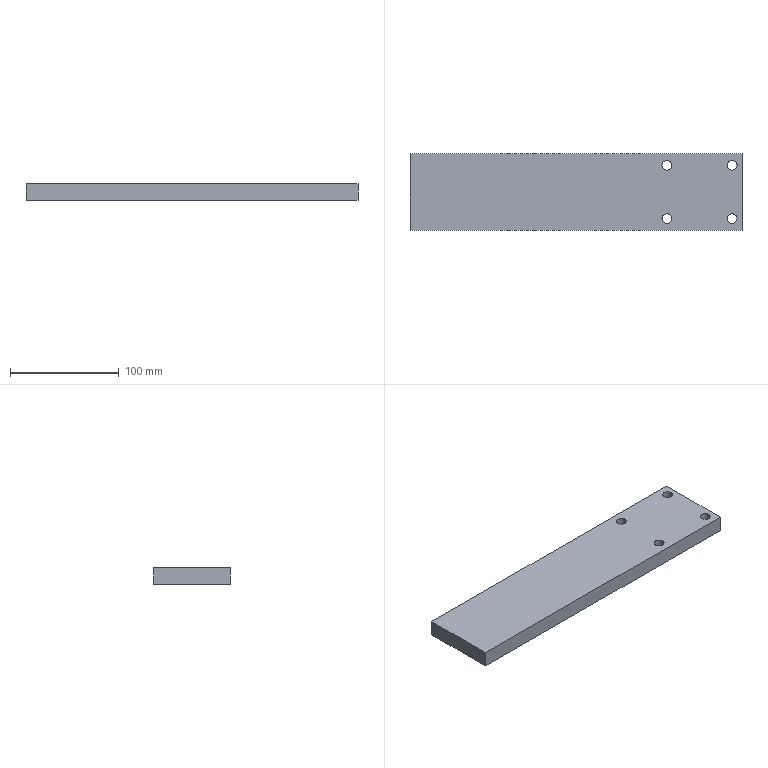Part | STEP file | Positioning_id1878_x_t | 1 solid | 14 faces | box 305 x 70 x 15 mm | volume 316433 mm3 | cylinder 8 | plane 6 | commonest cylinder face diameters 9 x8
STEP:
#1=CARTESIAN_POINT('',(0.,0.,0.));
#2=DIRECTION('',(0.,0.,1.));
#3=DIRECTION('',(1.,0.,0.));
#4=AXIS2_PLACEMENT_3D('',#1,#2,#3);
#5=CARTESIAN_POINT('',(-772.502,-24.5,534.5));
#6=VERTEX_POINT('',#5);
#7=CARTESIAN_POINT('',(-781.502,-24.5,534.5));
#8=VERTEX_POINT('',#7);
#9=CARTESIAN_POINT('',(-777.002,-24.5,534.5));
#10=DIRECTION('',(0.,0.,-1.));
#11=DIRECTION('',(-1.,0.,0.));
#12=AXIS2_PLACEMENT_3D('',#9,#10,#11);
#13=CIRCLE('',#12,4.5);
#14=CARTESIAN_POINT('',(-777.002,-24.5,454.5));
#15=DIRECTION('',(0.,0.,-1.));
#16=DIRECTION('',(1.,0.,0.));
#17=AXIS2_PLACEMENT_3D('',#14,#15,#16);
#18=CYLINDRICAL_SURFACE('',#17,4.5);
#19=CARTESIAN_POINT('',(-3.142,-80.));
#20=DIRECTION('',(1.,0.));
#21=VECTOR('',#20,1.);
#22=LINE('',#19,#21);
#23=(GEOMETRIC_REPRESENTATION_CONTEXT(2)PARAMETRIC_REPRESENTATION_CONTEXT()REPRESENTATION_CONTEXT('',''));
#24=DEFINITIONAL_REPRESENTATION('',(#22),#23);
#25=PCURVE('',#18,#24);
#26=CARTESIAN_POINT('',(-805.002,-37.5,534.5));
#27=DIRECTION('',(0.,0.,1.));
#28=DIRECTION('',(0.,-1.,0.));
#29=AXIS2_PLACEMENT_3D('',#26,#27,#28);
#30=PLANE('',#29);
#31=CARTESIAN_POINT('',(-13.,23.5));
#32=CARTESIAN_POINT('',(-20.794,23.5));
#33=CARTESIAN_POINT('',(-16.897,30.25));
#34=CARTESIAN_POINT('',(-13.,37.));
#35=CARTESIAN_POINT('',(-9.103,30.25));
#36=CARTESIAN_POINT('',(-5.206,23.5));
#37=CARTESIAN_POINT('',(-13.,23.5));
#38=(BOUNDED_CURVE()B_SPLINE_CURVE(2,(#31,#32,#33,#34,#35,#36,#37),.UNSPECIFIED.,.T.,.F.)B_SPLINE_CURVE_WITH_KNOTS((1,2,2,2,2,1),(-2.094,0.,2.094,4.189,6.283,8.378),.UNSPECIFIED.)CURVE()GEOMETRIC_REPRESENTATION_ITEM()RATIONAL_B_SPLINE_CURVE((1.,0.5,1.,0.5,1.,0.5,1.))REPRESENTATION_ITEM(''));
#39=(GEOMETRIC_REPRESENTATION_CONTEXT(2)PARAMETRIC_REPRESENTATION_CONTEXT()REPRESENTATION_CONTEXT('',''));
#40=DEFINITIONAL_REPRESENTATION('',(#38),#39);
#41=PCURVE('',#30,#40);
#42=SURFACE_CURVE('',#13,(#25,#41),.PCURVE_S1.);
#43=EDGE_CURVE('',#6,#8,#42,.T.);
#44=ORIENTED_EDGE('',*,*,#43,.T.);
#45=CARTESIAN_POINT('',(-781.502,-24.5,519.5));
#46=VERTEX_POINT('',#45);
#47=CARTESIAN_POINT('',(-781.502,-24.5,519.5));
#48=DIRECTION('',(0.,0.,1.));
#49=VECTOR('',#48,1.);
#50=LINE('',#47,#49);
#51=CARTESIAN_POINT('',(3.142,-65.));
#52=DIRECTION('',(0.,-1.));
#53=VECTOR('',#52,1.);
#54=LINE('',#51,#53);
#55=(GEOMETRIC_REPRESENTATION_CONTEXT(2)PARAMETRIC_REPRESENTATION_CONTEXT()REPRESENTATION_CONTEXT('',''));
#56=DEFINITIONAL_REPRESENTATION('',(#54),#55);
#57=PCURVE('',#18,#56);
#58=CARTESIAN_POINT('',(-777.002,-24.5,454.5));
#59=DIRECTION('',(0.,0.,-1.));
#60=DIRECTION('',(1.,0.,0.));
#61=AXIS2_PLACEMENT_3D('',#58,#59,#60);
#62=CYLINDRICAL_SURFACE('',#61,4.5);
#63=CARTESIAN_POINT('',(3.142,-65.));
#64=DIRECTION('',(0.,-1.));
#65=VECTOR('',#64,1.);
#66=LINE('',#63,#65);
#67=(GEOMETRIC_REPRESENTATION_CONTEXT(2)PARAMETRIC_REPRESENTATION_CONTEXT()REPRESENTATION_CONTEXT('',''));
#68=DEFINITIONAL_REPRESENTATION('',(#66),#67);
#69=PCURVE('',#62,#68);
#70=SURFACE_CURVE('',#50,(#57,#69),.PCURVE_S1.);
#71=EDGE_CURVE('',#46,#8,#70,.T.);
#72=ORIENTED_EDGE('',*,*,#71,.F.);
#73=CARTESIAN_POINT('',(-772.502,-24.5,519.5));
#74=VERTEX_POINT('',#73);
#75=CARTESIAN_POINT('',(-777.002,-24.5,519.5));
#76=DIRECTION('',(0.,0.,1.));
#77=DIRECTION('',(-1.,0.,0.));
#78=AXIS2_PLACEMENT_3D('',#75,#76,#77);
#79=CIRCLE('',#78,4.5);
#80=CARTESIAN_POINT('',(3.142,-65.));
#81=DIRECTION('',(-1.,0.));
#82=VECTOR('',#81,1.);
#83=LINE('',#80,#82);
#84=(GEOMETRIC_REPRESENTATION_CONTEXT(2)PARAMETRIC_REPRESENTATION_CONTEXT()REPRESENTATION_CONTEXT('',''));
#85=DEFINITIONAL_REPRESENTATION('',(#83),#84);
#86=PCURVE('',#18,#85);
#87=CARTESIAN_POINT('',(-805.002,-37.5,519.5));
#88=DIRECTION('',(0.,0.,-1.));
#89=DIRECTION('',(0.,1.,0.));
#90=AXIS2_PLACEMENT_3D('',#87,#88,#89);
#91=PLANE('',#90);
#92=CARTESIAN_POINT('',(13.,23.5));
#93=CARTESIAN_POINT('',(5.206,23.5));
#94=CARTESIAN_POINT('',(9.103,30.25));
#95=CARTESIAN_POINT('',(13.,37.));
#96=CARTESIAN_POINT('',(16.897,30.25));
#97=CARTESIAN_POINT('',(20.794,23.5));
#98=CARTESIAN_POINT('',(13.,23.5));
#99=(BOUNDED_CURVE()B_SPLINE_CURVE(2,(#92,#93,#94,#95,#96,#97,#98),.UNSPECIFIED.,.T.,.F.)B_SPLINE_CURVE_WITH_KNOTS((1,2,2,2,2,1),(-2.094,0.,2.094,4.189,6.283,8.378),.UNSPECIFIED.)CURVE()GEOMETRIC_REPRESENTATION_ITEM()RATIONAL_B_SPLINE_CURVE((1.,0.5,1.,0.5,1.,0.5,1.))REPRESENTATION_ITEM(''));
#100=(GEOMETRIC_REPRESENTATION_CONTEXT(2)PARAMETRIC_REPRESENTATION_CONTEXT()REPRESENTATION_CONTEXT('',''));
#101=DEFINITIONAL_REPRESENTATION('',(#99),#100);
#102=PCURVE('',#91,#101);
#103=SURFACE_CURVE('',#79,(#86,#102),.PCURVE_S1.);
#104=EDGE_CURVE('',#46,#74,#103,.T.);
#105=ORIENTED_EDGE('',*,*,#104,.T.);
#106=CARTESIAN_POINT('',(-772.502,-24.5,519.5));
#107=DIRECTION('',(0.,0.,-1.));
#108=VECTOR('',#107,1.);
#109=LINE('',#106,#108);
#110=CARTESIAN_POINT('',(0.,-65.));
#111=DIRECTION('',(0.,1.));
#112=VECTOR('',#111,1.);
#113=LINE('',#110,#112);
#114=(GEOMETRIC_REPRESENTATION_CONTEXT(2)PARAMETRIC_REPRESENTATION_CONTEXT()REPRESENTATION_CONTEXT('',''));
#115=DEFINITIONAL_REPRESENTATION('',(#113),#114);
#116=PCURVE('',#18,#115);
#117=CARTESIAN_POINT('',(6.283,-65.));
#118=DIRECTION('',(0.,1.));
#119=VECTOR('',#118,1.);
#120=LINE('',#117,#119);
#121=(GEOMETRIC_REPRESENTATION_CONTEXT(2)PARAMETRIC_REPRESENTATION_CONTEXT()REPRESENTATION_CONTEXT('',''));
#122=DEFINITIONAL_REPRESENTATION('',(#120),#121);
#123=PCURVE('',#62,#122);
#124=SURFACE_CURVE('',#109,(#116,#123),.PCURVE_S1.);
#125=EDGE_CURVE('',#6,#74,#124,.T.);
#126=ORIENTED_EDGE('',*,*,#125,.F.);
#127=EDGE_LOOP('',(#44,#72,#105,#126));
#128=FACE_BOUND('',#127,.F.);
#129=ADVANCED_FACE('',(#128),#18,.F.);
#130=CARTESIAN_POINT('',(-772.502,24.5,534.5));
#131=VERTEX_POINT('',#130);
#132=CARTESIAN_POINT('',(-781.502,24.5,534.5));
#133=VERTEX_POINT('',#132);
#134=CARTESIAN_POINT('',(-777.002,24.5,534.5));
#135=DIRECTION('',(0.,0.,-1.));
#136=DIRECTION('',(-1.,0.,0.));
#137=AXIS2_PLACEMENT_3D('',#134,#135,#136);
#138=CIRCLE('',#137,4.5);
#139=CARTESIAN_POINT('',(-777.002,24.5,454.5));
#140=DIRECTION('',(0.,0.,-1.));
#141=DIRECTION('',(1.,0.,0.));
#142=AXIS2_PLACEMENT_3D('',#139,#140,#141);
#143=CYLINDRICAL_SURFACE('',#142,4.5);
#144=CARTESIAN_POINT('',(-3.142,-80.));
#145=DIRECTION('',(1.,0.));
#146=VECTOR('',#145,1.);
#147=LINE('',#144,#146);
#148=(GEOMETRIC_REPRESENTATION_CONTEXT(2)PARAMETRIC_REPRESENTATION_CONTEXT()REPRESENTATION_CONTEXT('',''));
#149=DEFINITIONAL_REPRESENTATION('',(#147),#148);
#150=PCURVE('',#143,#149);
#151=CARTESIAN_POINT('',(-62.,23.5));
#152=CARTESIAN_POINT('',(-69.794,23.5));
#153=CARTESIAN_POINT('',(-65.897,30.25));
#154=CARTESIAN_POINT('',(-62.,37.));
#155=CARTESIAN_POINT('',(-58.103,30.25));
#156=CARTESIAN_POINT('',(-54.206,23.5));
#157=CARTESIAN_POINT('',(-62.,23.5));
#158=(BOUNDED_CURVE()B_SPLINE_CURVE(2,(#151,#152,#153,#154,#155,#156,#157),.UNSPECIFIED.,.T.,.F.)B_SPLINE_CURVE_WITH_KNOTS((1,2,2,2,2,1),(-2.094,0.,2.094,4.189,6.283,8.378),.UNSPECIFIED.)CURVE()GEOMETRIC_REPRESENTATION_ITEM()RATIONAL_B_SPLINE_CURVE((1.,0.5,1.,0.5,1.,0.5,1.))REPRESENTATION_ITEM(''));
#159=(GEOMETRIC_REPRESENTATION_CONTEXT(2)PARAMETRIC_REPRESENTATION_CONTEXT()REPRESENTATION_CONTEXT('',''));
#160=DEFINITIONAL_REPRESENTATION('',(#158),#159);
#161=PCURVE('',#30,#160);
#162=SURFACE_CURVE('',#138,(#150,#161),.PCURVE_S1.);
#163=EDGE_CURVE('',#131,#133,#162,.T.);
#164=ORIENTED_EDGE('',*,*,#163,.T.);
#165=CARTESIAN_POINT('',(-781.502,24.5,519.5));
#166=VERTEX_POINT('',#165);
#167=CARTESIAN_POINT('',(-781.502,24.5,519.5));
#168=DIRECTION('',(0.,0.,-1.));
#169=VECTOR('',#168,1.);
#170=LINE('',#167,#169);
#171=CARTESIAN_POINT('',(3.142,-65.));
#172=DIRECTION('',(0.,1.));
#173=VECTOR('',#172,1.);
#174=LINE('',#171,#173);
#175=(GEOMETRIC_REPRESENTATION_CONTEXT(2)PARAMETRIC_REPRESENTATION_CONTEXT()REPRESENTATION_CONTEXT('',''));
#176=DEFINITIONAL_REPRESENTATION('',(#174),#175);
#177=PCURVE('',#143,#176);
#178=CARTESIAN_POINT('',(-777.002,24.5,454.5));
#179=DIRECTION('',(0.,0.,-1.));
#180=DIRECTION('',(1.,0.,0.));
#181=AXIS2_PLACEMENT_3D('',#178,#179,#180);
#182=CYLINDRICAL_SURFACE('',#181,4.5);
#183=CARTESIAN_POINT('',(3.142,-65.));
#184=DIRECTION('',(0.,1.));
#185=VECTOR('',#184,1.);
#186=LINE('',#183,#185);
#187=(GEOMETRIC_REPRESENTATION_CONTEXT(2)PARAMETRIC_REPRESENTATION_CONTEXT()REPRESENTATION_CONTEXT('',''));
#188=DEFINITIONAL_REPRESENTATION('',(#186),#187);
#189=PCURVE('',#182,#188);
#190=SURFACE_CURVE('',#170,(#177,#189),.PCURVE_S1.);
#191=EDGE_CURVE('',#133,#166,#190,.T.);
#192=ORIENTED_EDGE('',*,*,#191,.T.);
#193=CARTESIAN_POINT('',(-772.502,24.5,519.5));
#194=VERTEX_POINT('',#193);
#195=CARTESIAN_POINT('',(-777.002,24.5,519.5));
#196=DIRECTION('',(0.,0.,1.));
#197=DIRECTION('',(-1.,0.,0.));
#198=AXIS2_PLACEMENT_3D('',#195,#196,#197);
#199=CIRCLE('',#198,4.5);
#200=CARTESIAN_POINT('',(3.142,-65.));
#201=DIRECTION('',(-1.,0.));
#202=VECTOR('',#201,1.);
#203=LINE('',#200,#202);
#204=(GEOMETRIC_REPRESENTATION_CONTEXT(2)PARAMETRIC_REPRESENTATION_CONTEXT()REPRESENTATION_CONTEXT('',''));
#205=DEFINITIONAL_REPRESENTATION('',(#203),#204);
#206=PCURVE('',#143,#205);
#207=CARTESIAN_POINT('',(62.,23.5));
#208=CARTESIAN_POINT('',(54.206,23.5));
#209=CARTESIAN_POINT('',(58.103,30.25));
#210=CARTESIAN_POINT('',(62.,37.));
#211=CARTESIAN_POINT('',(65.897,30.25));
#212=CARTESIAN_POINT('',(69.794,23.5));
#213=CARTESIAN_POINT('',(62.,23.5));
#214=(BOUNDED_CURVE()B_SPLINE_CURVE(2,(#207,#208,#209,#210,#211,#212,#213),.UNSPECIFIED.,.T.,.F.)B_SPLINE_CURVE_WITH_KNOTS((1,2,2,2,2,1),(-2.094,0.,2.094,4.189,6.283,8.378),.UNSPECIFIED.)CURVE()GEOMETRIC_REPRESENTATION_ITEM()RATIONAL_B_SPLINE_CURVE((1.,0.5,1.,0.5,1.,0.5,1.))REPRESENTATION_ITEM(''));
#215=(GEOMETRIC_REPRESENTATION_CONTEXT(2)PARAMETRIC_REPRESENTATION_CONTEXT()REPRESENTATION_CONTEXT('',''));
#216=DEFINITIONAL_REPRESENTATION('',(#214),#215);
#217=PCURVE('',#91,#216);
#218=SURFACE_CURVE('',#199,(#206,#217),.PCURVE_S1.);
#219=EDGE_CURVE('',#166,#194,#218,.T.);
#220=ORIENTED_EDGE('',*,*,#219,.T.);
#221=CARTESIAN_POINT('',(-772.502,24.5,519.5));
#222=DIRECTION('',(0.,0.,1.));
#223=VECTOR('',#222,1.);
#224=LINE('',#221,#223);
#225=CARTESIAN_POINT('',(0.,-65.));
#226=DIRECTION('',(0.,-1.));
#227=VECTOR('',#226,1.);
#228=LINE('',#225,#227);
#229=(GEOMETRIC_REPRESENTATION_CONTEXT(2)PARAMETRIC_REPRESENTATION_CONTEXT()REPRESENTATION_CONTEXT('',''));
#230=DEFINITIONAL_REPRESENTATION('',(#228),#229);
#231=PCURVE('',#143,#230);
#232=CARTESIAN_POINT('',(6.283,-65.));
#233=DIRECTION('',(0.,-1.));
#234=VECTOR('',#233,1.);
#235=LINE('',#232,#234);
#236=(GEOMETRIC_REPRESENTATION_CONTEXT(2)PARAMETRIC_REPRESENTATION_CONTEXT()REPRESENTATION_CONTEXT('',''));
#237=DEFINITIONAL_REPRESENTATION('',(#235),#236);
#238=PCURVE('',#182,#237);
#239=SURFACE_CURVE('',#224,(#231,#238),.PCURVE_S1.);
#240=EDGE_CURVE('',#194,#131,#239,.T.);
#241=ORIENTED_EDGE('',*,*,#240,.T.);
#242=EDGE_LOOP('',(#164,#192,#220,#241));
#243=FACE_BOUND('',#242,.F.);
#244=ADVANCED_FACE('',(#243),#143,.F.);
#245=CARTESIAN_POINT('',(-712.502,24.5,534.5));
#246=VERTEX_POINT('',#245);
#247=CARTESIAN_POINT('',(-721.502,24.5,534.5));
#248=VERTEX_POINT('',#247);
#249=CARTESIAN_POINT('',(-717.002,24.5,534.5));
#250=DIRECTION('',(0.,0.,-1.));
#251=DIRECTION('',(-1.,0.,0.));
#252=AXIS2_PLACEMENT_3D('',#249,#250,#251);
#253=CIRCLE('',#252,4.5);
#254=CARTESIAN_POINT('',(-717.002,24.5,454.5));
#255=DIRECTION('',(0.,0.,-1.));
#256=DIRECTION('',(1.,0.,0.));
#257=AXIS2_PLACEMENT_3D('',#254,#255,#256);
#258=CYLINDRICAL_SURFACE('',#257,4.5);
#259=CARTESIAN_POINT('',(-3.142,-80.));
#260=DIRECTION('',(1.,0.));
#261=VECTOR('',#260,1.);
#262=LINE('',#259,#261);
#263=(GEOMETRIC_REPRESENTATION_CONTEXT(2)PARAMETRIC_REPRESENTATION_CONTEXT()REPRESENTATION_CONTEXT('',''));
#264=DEFINITIONAL_REPRESENTATION('',(#262),#263);
#265=PCURVE('',#258,#264);
#266=CARTESIAN_POINT('',(-62.,83.5));
#267=CARTESIAN_POINT('',(-69.794,83.5));
#268=CARTESIAN_POINT('',(-65.897,90.25));
#269=CARTESIAN_POINT('',(-62.,97.));
#270=CARTESIAN_POINT('',(-58.103,90.25));
#271=CARTESIAN_POINT('',(-54.206,83.5));
#272=CARTESIAN_POINT('',(-62.,83.5));
#273=(BOUNDED_CURVE()B_SPLINE_CURVE(2,(#266,#267,#268,#269,#270,#271,#272),.UNSPECIFIED.,.T.,.F.)B_SPLINE_CURVE_WITH_KNOTS((1,2,2,2,2,1),(-2.094,0.,2.094,4.189,6.283,8.378),.UNSPECIFIED.)CURVE()GEOMETRIC_REPRESENTATION_ITEM()RATIONAL_B_SPLINE_CURVE((1.,0.5,1.,0.5,1.,0.5,1.))REPRESENTATION_ITEM(''));
#274=(GEOMETRIC_REPRESENTATION_CONTEXT(2)PARAMETRIC_REPRESENTATION_CONTEXT()REPRESENTATION_CONTEXT('',''));
#275=DEFINITIONAL_REPRESENTATION('',(#273),#274);
#276=PCURVE('',#30,#275);
#277=SURFACE_CURVE('',#253,(#265,#276),.PCURVE_S1.);
#278=EDGE_CURVE('',#246,#248,#277,.T.);
#279=ORIENTED_EDGE('',*,*,#278,.T.);
#280=CARTESIAN_POINT('',(-721.502,24.5,519.5));
#281=VERTEX_POINT('',#280);
#282=CARTESIAN_POINT('',(-721.502,24.5,519.5));
#283=DIRECTION('',(0.,0.,-1.));
#284=VECTOR('',#283,1.);
#285=LINE('',#282,#284);
#286=CARTESIAN_POINT('',(3.142,-65.));
#287=DIRECTION('',(0.,1.));
#288=VECTOR('',#287,1.);
#289=LINE('',#286,#288);
#290=(GEOMETRIC_REPRESENTATION_CONTEXT(2)PARAMETRIC_REPRESENTATION_CONTEXT()REPRESENTATION_CONTEXT('',''));
#291=DEFINITIONAL_REPRESENTATION('',(#289),#290);
#292=PCURVE('',#258,#291);
#293=CARTESIAN_POINT('',(-717.002,24.5,454.5));
#294=DIRECTION('',(0.,0.,-1.));
#295=DIRECTION('',(1.,0.,0.));
#296=AXIS2_PLACEMENT_3D('',#293,#294,#295);
#297=CYLINDRICAL_SURFACE('',#296,4.5);
#298=CARTESIAN_POINT('',(3.142,-65.));
#299=DIRECTION('',(0.,1.));
#300=VECTOR('',#299,1.);
#301=LINE('',#298,#300);
#302=(GEOMETRIC_REPRESENTATION_CONTEXT(2)PARAMETRIC_REPRESENTATION_CONTEXT()REPRESENTATION_CONTEXT('',''));
#303=DEFINITIONAL_REPRESENTATION('',(#301),#302);
#304=PCURVE('',#297,#303);
#305=SURFACE_CURVE('',#285,(#292,#304),.PCURVE_S1.);
#306=EDGE_CURVE('',#248,#281,#305,.T.);
#307=ORIENTED_EDGE('',*,*,#306,.T.);
#308=CARTESIAN_POINT('',(-712.502,24.5,519.5));
#309=VERTEX_POINT('',#308);
#310=CARTESIAN_POINT('',(-717.002,24.5,519.5));
#311=DIRECTION('',(0.,0.,1.));
#312=DIRECTION('',(-1.,0.,0.));
#313=AXIS2_PLACEMENT_3D('',#310,#311,#312);
#314=CIRCLE('',#313,4.5);
#315=CARTESIAN_POINT('',(3.142,-65.));
#316=DIRECTION('',(-1.,0.));
#317=VECTOR('',#316,1.);
#318=LINE('',#315,#317);
#319=(GEOMETRIC_REPRESENTATION_CONTEXT(2)PARAMETRIC_REPRESENTATION_CONTEXT()REPRESENTATION_CONTEXT('',''));
#320=DEFINITIONAL_REPRESENTATION('',(#318),#319);
#321=PCURVE('',#258,#320);
#322=CARTESIAN_POINT('',(62.,83.5));
#323=CARTESIAN_POINT('',(54.206,83.5));
#324=CARTESIAN_POINT('',(58.103,90.25));
#325=CARTESIAN_POINT('',(62.,97.));
#326=CARTESIAN_POINT('',(65.897,90.25));
#327=CARTESIAN_POINT('',(69.794,83.5));
#328=CARTESIAN_POINT('',(62.,83.5));
#329=(BOUNDED_CURVE()B_SPLINE_CURVE(2,(#322,#323,#324,#325,#326,#327,#328),.UNSPECIFIED.,.T.,.F.)B_SPLINE_CURVE_WITH_KNOTS((1,2,2,2,2,1),(-2.094,0.,2.094,4.189,6.283,8.378),.UNSPECIFIED.)CURVE()GEOMETRIC_REPRESENTATION_ITEM()RATIONAL_B_SPLINE_CURVE((1.,0.5,1.,0.5,1.,0.5,1.))REPRESENTATION_ITEM(''));
#330=(GEOMETRIC_REPRESENTATION_CONTEXT(2)PARAMETRIC_REPRESENTATION_CONTEXT()REPRESENTATION_CONTEXT('',''));
#331=DEFINITIONAL_REPRESENTATION('',(#329),#330);
#332=PCURVE('',#91,#331);
#333=SURFACE_CURVE('',#314,(#321,#332),.PCURVE_S1.);
#334=EDGE_CURVE('',#281,#309,#333,.T.);
#335=ORIENTED_EDGE('',*,*,#334,.T.);
#336=CARTESIAN_POINT('',(-712.502,24.5,519.5));
#337=DIRECTION('',(0.,0.,1.));
#338=VECTOR('',#337,1.);
#339=LINE('',#336,#338);
#340=CARTESIAN_POINT('',(0.,-65.));
#341=DIRECTION('',(0.,-1.));
#342=VECTOR('',#341,1.);
#343=LINE('',#340,#342);
#344=(GEOMETRIC_REPRESENTATION_CONTEXT(2)PARAMETRIC_REPRESENTATION_CONTEXT()REPRESENTATION_CONTEXT('',''));
#345=DEFINITIONAL_REPRESENTATION('',(#343),#344);
#346=PCURVE('',#258,#345);
#347=CARTESIAN_POINT('',(6.283,-65.));
#348=DIRECTION('',(0.,-1.));
#349=VECTOR('',#348,1.);
#350=LINE('',#347,#349);
#351=(GEOMETRIC_REPRESENTATION_CONTEXT(2)PARAMETRIC_REPRESENTATION_CONTEXT()REPRESENTATION_CONTEXT('',''));
#352=DEFINITIONAL_REPRESENTATION('',(#350),#351);
#353=PCURVE('',#297,#352);
#354=SURFACE_CURVE('',#339,(#346,#353),.PCURVE_S1.);
#355=EDGE_CURVE('',#309,#246,#354,.T.);
#356=ORIENTED_EDGE('',*,*,#355,.T.);
#357=EDGE_LOOP('',(#279,#307,#335,#356));
#358=FACE_BOUND('',#357,.F.);
#359=ADVANCED_FACE('',(#358),#258,.F.);
#360=CARTESIAN_POINT('',(-712.502,-24.5,534.5));
#361=VERTEX_POINT('',#360);
#362=CARTESIAN_POINT('',(-721.502,-24.5,534.5));
#363=VERTEX_POINT('',#362);
#364=CARTESIAN_POINT('',(-717.002,-24.5,534.5));
#365=DIRECTION('',(0.,0.,-1.));
#366=DIRECTION('',(-1.,0.,0.));
#367=AXIS2_PLACEMENT_3D('',#364,#365,#366);
#368=CIRCLE('',#367,4.5);
#369=CARTESIAN_POINT('',(-717.002,-24.5,454.5));
#370=DIRECTION('',(0.,0.,-1.));
#371=DIRECTION('',(1.,0.,0.));
#372=AXIS2_PLACEMENT_3D('',#369,#370,#371);
#373=CYLINDRICAL_SURFACE('',#372,4.5);
#374=CARTESIAN_POINT('',(-3.142,-80.));
#375=DIRECTION('',(1.,0.));
#376=VECTOR('',#375,1.);
#377=LINE('',#374,#376);
#378=(GEOMETRIC_REPRESENTATION_CONTEXT(2)PARAMETRIC_REPRESENTATION_CONTEXT()REPRESENTATION_CONTEXT('',''));
#379=DEFINITIONAL_REPRESENTATION('',(#377),#378);
#380=PCURVE('',#373,#379);
#381=CARTESIAN_POINT('',(-13.,83.5));
#382=CARTESIAN_POINT('',(-20.794,83.5));
#383=CARTESIAN_POINT('',(-16.897,90.25));
#384=CARTESIAN_POINT('',(-13.,97.));
#385=CARTESIAN_POINT('',(-9.103,90.25));
#386=CARTESIAN_POINT('',(-5.206,83.5));
#387=CARTESIAN_POINT('',(-13.,83.5));
#388=(BOUNDED_CURVE()B_SPLINE_CURVE(2,(#381,#382,#383,#384,#385,#386,#387),.UNSPECIFIED.,.T.,.F.)B_SPLINE_CURVE_WITH_KNOTS((1,2,2,2,2,1),(-2.094,0.,2.094,4.189,6.283,8.378),.UNSPECIFIED.)CURVE()GEOMETRIC_REPRESENTATION_ITEM()RATIONAL_B_SPLINE_CURVE((1.,0.5,1.,0.5,1.,0.5,1.))REPRESENTATION_ITEM(''));
#389=(GEOMETRIC_REPRESENTATION_CONTEXT(2)PARAMETRIC_REPRESENTATION_CONTEXT()REPRESENTATION_CONTEXT('',''));
#390=DEFINITIONAL_REPRESENTATION('',(#388),#389);
#391=PCURVE('',#30,#390);
#392=SURFACE_CURVE('',#368,(#380,#391),.PCURVE_S1.);
#393=EDGE_CURVE('',#361,#363,#392,.T.);
#394=ORIENTED_EDGE('',*,*,#393,.T.);
#395=CARTESIAN_POINT('',(-721.502,-24.5,519.5));
#396=VERTEX_POINT('',#395);
#397=CARTESIAN_POINT('',(-721.502,-24.5,519.5));
#398=DIRECTION('',(0.,0.,1.));
#399=VECTOR('',#398,1.);
#400=LINE('',#397,#399);
#401=CARTESIAN_POINT('',(3.142,-65.));
#402=DIRECTION('',(0.,-1.));
#403=VECTOR('',#402,1.);
#404=LINE('',#401,#403);
#405=(GEOMETRIC_REPRESENTATION_CONTEXT(2)PARAMETRIC_REPRESENTATION_CONTEXT()REPRESENTATION_CONTEXT('',''));
#406=DEFINITIONAL_REPRESENTATION('',(#404),#405);
#407=PCURVE('',#373,#406);
#408=CARTESIAN_POINT('',(-717.002,-24.5,454.5));
#409=DIRECTION('',(0.,0.,-1.));
#410=DIRECTION('',(1.,0.,0.));
#411=AXIS2_PLACEMENT_3D('',#408,#409,#410);
#412=CYLINDRICAL_SURFACE('',#411,4.5);
#413=CARTESIAN_POINT('',(3.142,-65.));
#414=DIRECTION('',(0.,-1.));
#415=VECTOR('',#414,1.);
#416=LINE('',#413,#415);
#417=(GEOMETRIC_REPRESENTATION_CONTEXT(2)PARAMETRIC_REPRESENTATION_CONTEXT()REPRESENTATION_CONTEXT('',''));
#418=DEFINITIONAL_REPRESENTATION('',(#416),#417);
#419=PCURVE('',#412,#418);
#420=SURFACE_CURVE('',#400,(#407,#419),.PCURVE_S1.);
#421=EDGE_CURVE('',#396,#363,#420,.T.);
#422=ORIENTED_EDGE('',*,*,#421,.F.);
#423=CARTESIAN_POINT('',(-712.502,-24.5,519.5));
#424=VERTEX_POINT('',#423);
#425=CARTESIAN_POINT('',(-717.002,-24.5,519.5));
#426=DIRECTION('',(0.,0.,1.));
#427=DIRECTION('',(-1.,0.,0.));
#428=AXIS2_PLACEMENT_3D('',#425,#426,#427);
#429=CIRCLE('',#428,4.5);
#430=CARTESIAN_POINT('',(3.142,-65.));
#431=DIRECTION('',(-1.,0.));
#432=VECTOR('',#431,1.);
#433=LINE('',#430,#432);
#434=(GEOMETRIC_REPRESENTATION_CONTEXT(2)PARAMETRIC_REPRESENTATION_CONTEXT()REPRESENTATION_CONTEXT('',''));
#435=DEFINITIONAL_REPRESENTATION('',(#433),#434);
#436=PCURVE('',#373,#435);
#437=CARTESIAN_POINT('',(13.,83.5));
#438=CARTESIAN_POINT('',(5.206,83.5));
#439=CARTESIAN_POINT('',(9.103,90.25));
#440=CARTESIAN_POINT('',(13.,97.));
#441=CARTESIAN_POINT('',(16.897,90.25));
#442=CARTESIAN_POINT('',(20.794,83.5));
#443=CARTESIAN_POINT('',(13.,83.5));
#444=(BOUNDED_CURVE()B_SPLINE_CURVE(2,(#437,#438,#439,#440,#441,#442,#443),.UNSPECIFIED.,.T.,.F.)B_SPLINE_CURVE_WITH_KNOTS((1,2,2,2,2,1),(-2.094,0.,2.094,4.189,6.283,8.378),.UNSPECIFIED.)CURVE()GEOMETRIC_REPRESENTATION_ITEM()RATIONAL_B_SPLINE_CURVE((1.,0.5,1.,0.5,1.,0.5,1.))REPRESENTATION_ITEM(''));
#445=(GEOMETRIC_REPRESENTATION_CONTEXT(2)PARAMETRIC_REPRESENTATION_CONTEXT()REPRESENTATION_CONTEXT('',''));
#446=DEFINITIONAL_REPRESENTATION('',(#444),#445);
#447=PCURVE('',#91,#446);
#448=SURFACE_CURVE('',#429,(#436,#447),.PCURVE_S1.);
#449=EDGE_CURVE('',#396,#424,#448,.T.);
#450=ORIENTED_EDGE('',*,*,#449,.T.);
#451=CARTESIAN_POINT('',(-712.502,-24.5,519.5));
#452=DIRECTION('',(0.,0.,-1.));
#453=VECTOR('',#452,1.);
#454=LINE('',#451,#453);
#455=CARTESIAN_POINT('',(0.,-65.));
#456=DIRECTION('',(0.,1.));
#457=VECTOR('',#456,1.);
#458=LINE('',#455,#457);
#459=(GEOMETRIC_REPRESENTATION_CONTEXT(2)PARAMETRIC_REPRESENTATION_CONTEXT()REPRESENTATION_CONTEXT('',''));
#460=DEFINITIONAL_REPRESENTATION('',(#458),#459);
#461=PCURVE('',#373,#460);
#462=CARTESIAN_POINT('',(6.283,-65.));
#463=DIRECTION('',(0.,1.));
#464=VECTOR('',#463,1.);
#465=LINE('',#462,#464);
#466=(GEOMETRIC_REPRESENTATION_CONTEXT(2)PARAMETRIC_REPRESENTATION_CONTEXT()REPRESENTATION_CONTEXT('',''));
#467=DEFINITIONAL_REPRESENTATION('',(#465),#466);
#468=PCURVE('',#412,#467);
#469=SURFACE_CURVE('',#454,(#461,#468),.PCURVE_S1.);
#470=EDGE_CURVE('',#361,#424,#469,.T.);
#471=ORIENTED_EDGE('',*,*,#470,.F.);
#472=EDGE_LOOP('',(#394,#422,#450,#471));
#473=FACE_BOUND('',#472,.F.);
#474=ADVANCED_FACE('',(#473),#373,.F.);
#475=CARTESIAN_POINT('',(-1013.002,35.,519.5));
#476=VERTEX_POINT('',#475);
#477=CARTESIAN_POINT('',(-1013.002,35.,534.5));
#478=VERTEX_POINT('',#477);
#479=CARTESIAN_POINT('',(-1013.002,35.,519.5));
#480=DIRECTION('',(0.,0.,1.));
#481=VECTOR('',#480,1.);
#482=LINE('',#479,#481);
#483=CARTESIAN_POINT('',(-1013.002,-296.75,174.));
#484=DIRECTION('',(1.,0.,0.));
#485=DIRECTION('',(0.,1.,0.));
#486=AXIS2_PLACEMENT_3D('',#483,#484,#485);
#487=PLANE('',#486);
#488=CARTESIAN_POINT('',(331.75,345.5));
#489=DIRECTION('',(0.,1.));
#490=VECTOR('',#489,1.);
#491=LINE('',#488,#490);
#492=(GEOMETRIC_REPRESENTATION_CONTEXT(2)PARAMETRIC_REPRESENTATION_CONTEXT()REPRESENTATION_CONTEXT('',''));
#493=DEFINITIONAL_REPRESENTATION('',(#491),#492);
#494=PCURVE('',#487,#493);
#495=CARTESIAN_POINT('',(-805.002,35.,549.5));
#496=DIRECTION('',(0.,1.,0.));
#497=DIRECTION('',(-1.,0.,0.));
#498=AXIS2_PLACEMENT_3D('',#495,#496,#497);
#499=PLANE('',#498);
#500=CARTESIAN_POINT('',(208.,-30.));
#501=DIRECTION('',(0.,1.));
#502=VECTOR('',#501,1.);
#503=LINE('',#500,#502);
#504=(GEOMETRIC_REPRESENTATION_CONTEXT(2)PARAMETRIC_REPRESENTATION_CONTEXT()REPRESENTATION_CONTEXT('',''));
#505=DEFINITIONAL_REPRESENTATION('',(#503),#504);
#506=PCURVE('',#499,#505);
#507=SURFACE_CURVE('',#482,(#494,#506),.PCURVE_S1.);
#508=EDGE_CURVE('',#476,#478,#507,.T.);
#509=ORIENTED_EDGE('',*,*,#508,.F.);
#510=CARTESIAN_POINT('',(-1013.002,-35.,519.5));
#511=VERTEX_POINT('',#510);
#512=CARTESIAN_POINT('',(-1013.002,-35.,519.5));
#513=DIRECTION('',(0.,1.,0.));
#514=VECTOR('',#513,1.);
#515=LINE('',#512,#514);
#516=CARTESIAN_POINT('',(261.75,345.5));
#517=DIRECTION('',(1.,0.));
#518=VECTOR('',#517,1.);
#519=LINE('',#516,#518);
#520=(GEOMETRIC_REPRESENTATION_CONTEXT(2)PARAMETRIC_REPRESENTATION_CONTEXT()REPRESENTATION_CONTEXT('',''));
#521=DEFINITIONAL_REPRESENTATION('',(#519),#520);
#522=PCURVE('',#487,#521);
#523=CARTESIAN_POINT('',(2.5,-208.));
#524=DIRECTION('',(1.,0.));
#525=VECTOR('',#524,1.);
#526=LINE('',#523,#525);
#527=(GEOMETRIC_REPRESENTATION_CONTEXT(2)PARAMETRIC_REPRESENTATION_CONTEXT()REPRESENTATION_CONTEXT('',''));
#528=DEFINITIONAL_REPRESENTATION('',(#526),#527);
#529=PCURVE('',#91,#528);
#530=SURFACE_CURVE('',#515,(#522,#529),.PCURVE_S1.);
#531=EDGE_CURVE('',#511,#476,#530,.T.);
#532=ORIENTED_EDGE('',*,*,#531,.F.);
#533=CARTESIAN_POINT('',(-1013.002,-35.,534.5));
#534=VERTEX_POINT('',#533);
#535=CARTESIAN_POINT('',(-1013.002,-35.,534.5));
#536=DIRECTION('',(0.,0.,-1.));
#537=VECTOR('',#536,1.);
#538=LINE('',#535,#537);
#539=CARTESIAN_POINT('',(261.75,360.5));
#540=DIRECTION('',(0.,-1.));
#541=VECTOR('',#540,1.);
#542=LINE('',#539,#541);
#543=(GEOMETRIC_REPRESENTATION_CONTEXT(2)PARAMETRIC_REPRESENTATION_CONTEXT()REPRESENTATION_CONTEXT('',''));
#544=DEFINITIONAL_REPRESENTATION('',(#542),#543);
#545=PCURVE('',#487,#544);
#546=CARTESIAN_POINT('',(-805.002,-35.,549.5));
#547=DIRECTION('',(0.,-1.,0.));
#548=DIRECTION('',(1.,0.,0.));
#549=AXIS2_PLACEMENT_3D('',#546,#547,#548);
#550=PLANE('',#549);
#551=CARTESIAN_POINT('',(-208.,-15.));
#552=DIRECTION('',(0.,-1.));
#553=VECTOR('',#552,1.);
#554=LINE('',#551,#553);
#555=(GEOMETRIC_REPRESENTATION_CONTEXT(2)PARAMETRIC_REPRESENTATION_CONTEXT()REPRESENTATION_CONTEXT('',''));
#556=DEFINITIONAL_REPRESENTATION('',(#554),#555);
#557=PCURVE('',#550,#556);
#558=SURFACE_CURVE('',#538,(#545,#557),.PCURVE_S1.);
#559=EDGE_CURVE('',#534,#511,#558,.T.);
#560=ORIENTED_EDGE('',*,*,#559,.F.);
#561=CARTESIAN_POINT('',(-1013.002,35.,534.5));
#562=DIRECTION('',(0.,-1.,0.));
#563=VECTOR('',#562,1.);
#564=LINE('',#561,#563);
#565=CARTESIAN_POINT('',(331.75,360.5));
#566=DIRECTION('',(-1.,0.));
#567=VECTOR('',#566,1.);
#568=LINE('',#565,#567);
#569=(GEOMETRIC_REPRESENTATION_CONTEXT(2)PARAMETRIC_REPRESENTATION_CONTEXT()REPRESENTATION_CONTEXT('',''));
#570=DEFINITIONAL_REPRESENTATION('',(#568),#569);
#571=PCURVE('',#487,#570);
#572=CARTESIAN_POINT('',(-72.5,-208.));
#573=DIRECTION('',(1.,0.));
#574=VECTOR('',#573,1.);
#575=LINE('',#572,#574);
#576=(GEOMETRIC_REPRESENTATION_CONTEXT(2)PARAMETRIC_REPRESENTATION_CONTEXT()REPRESENTATION_CONTEXT('',''));
#577=DEFINITIONAL_REPRESENTATION('',(#575),#576);
#578=PCURVE('',#30,#577);
#579=SURFACE_CURVE('',#564,(#571,#578),.PCURVE_S1.);
#580=EDGE_CURVE('',#478,#534,#579,.T.);
#581=ORIENTED_EDGE('',*,*,#580,.F.);
#582=EDGE_LOOP('',(#509,#532,#560,#581));
#583=FACE_BOUND('',#582,.T.);
#584=ADVANCED_FACE('',(#583),#487,.F.);
#585=CARTESIAN_POINT('',(-708.002,-35.,534.5));
#586=VERTEX_POINT('',#585);
#587=CARTESIAN_POINT('',(-708.002,-35.,519.5));
#588=VERTEX_POINT('',#587);
#589=CARTESIAN_POINT('',(-708.002,-35.,534.5));
#590=DIRECTION('',(0.,0.,-1.));
#591=VECTOR('',#590,1.);
#592=LINE('',#589,#591);
#593=CARTESIAN_POINT('',(-708.002,-37.5,549.5));
#594=DIRECTION('',(1.,0.,0.));
#595=DIRECTION('',(0.,1.,0.));
#596=AXIS2_PLACEMENT_3D('',#593,#594,#595);
#597=PLANE('',#596);
#598=CARTESIAN_POINT('',(2.5,-15.));
#599=DIRECTION('',(0.,-1.));
#600=VECTOR('',#599,1.);
#601=LINE('',#598,#600);
#602=(GEOMETRIC_REPRESENTATION_CONTEXT(2)PARAMETRIC_REPRESENTATION_CONTEXT()REPRESENTATION_CONTEXT('',''));
#603=DEFINITIONAL_REPRESENTATION('',(#601),#602);
#604=PCURVE('',#597,#603);
#605=CARTESIAN_POINT('',(97.,-15.));
#606=DIRECTION('',(0.,-1.));
#607=VECTOR('',#606,1.);
#608=LINE('',#605,#607);
#609=(GEOMETRIC_REPRESENTATION_CONTEXT(2)PARAMETRIC_REPRESENTATION_CONTEXT()REPRESENTATION_CONTEXT('',''));
#610=DEFINITIONAL_REPRESENTATION('',(#608),#609);
#611=PCURVE('',#550,#610);
#612=SURFACE_CURVE('',#592,(#604,#611),.PCURVE_S1.);
#613=EDGE_CURVE('',#586,#588,#612,.T.);
#614=ORIENTED_EDGE('',*,*,#613,.T.);
#615=CARTESIAN_POINT('',(-708.002,35.,519.5));
#616=VERTEX_POINT('',#615);
#617=CARTESIAN_POINT('',(-708.002,-35.,519.5));
#618=DIRECTION('',(0.,1.,0.));
#619=VECTOR('',#618,1.);
#620=LINE('',#617,#619);
#621=CARTESIAN_POINT('',(2.5,-30.));
#622=DIRECTION('',(1.,0.));
#623=VECTOR('',#622,1.);
#624=LINE('',#621,#623);
#625=(GEOMETRIC_REPRESENTATION_CONTEXT(2)PARAMETRIC_REPRESENTATION_CONTEXT()REPRESENTATION_CONTEXT('',''));
#626=DEFINITIONAL_REPRESENTATION('',(#624),#625);
#627=PCURVE('',#597,#626);
#628=CARTESIAN_POINT('',(2.5,97.));
#629=DIRECTION('',(1.,0.));
#630=VECTOR('',#629,1.);
#631=LINE('',#628,#630);
#632=(GEOMETRIC_REPRESENTATION_CONTEXT(2)PARAMETRIC_REPRESENTATION_CONTEXT()REPRESENTATION_CONTEXT('',''));
#633=DEFINITIONAL_REPRESENTATION('',(#631),#632);
#634=PCURVE('',#91,#633);
#635=SURFACE_CURVE('',#620,(#627,#634),.PCURVE_S1.);
#636=EDGE_CURVE('',#588,#616,#635,.T.);
#637=ORIENTED_EDGE('',*,*,#636,.T.);
#638=CARTESIAN_POINT('',(-708.002,35.,534.5));
#639=VERTEX_POINT('',#638);
#640=CARTESIAN_POINT('',(-708.002,35.,534.5));
#641=DIRECTION('',(0.,0.,-1.));
#642=VECTOR('',#641,1.);
#643=LINE('',#640,#642);
#644=CARTESIAN_POINT('',(72.5,-15.));
#645=DIRECTION('',(0.,-1.));
#646=VECTOR('',#645,1.);
#647=LINE('',#644,#646);
#648=(GEOMETRIC_REPRESENTATION_CONTEXT(2)PARAMETRIC_REPRESENTATION_CONTEXT()REPRESENTATION_CONTEXT('',''));
#649=DEFINITIONAL_REPRESENTATION('',(#647),#648);
#650=PCURVE('',#597,#649);
#651=CARTESIAN_POINT('',(-97.,-15.));
#652=DIRECTION('',(0.,-1.));
#653=VECTOR('',#652,1.);
#654=LINE('',#651,#653);
#655=(GEOMETRIC_REPRESENTATION_CONTEXT(2)PARAMETRIC_REPRESENTATION_CONTEXT()REPRESENTATION_CONTEXT('',''));
#656=DEFINITIONAL_REPRESENTATION('',(#654),#655);
#657=PCURVE('',#499,#656);
#658=SURFACE_CURVE('',#643,(#650,#657),.PCURVE_S1.);
#659=EDGE_CURVE('',#639,#616,#658,.T.);
#660=ORIENTED_EDGE('',*,*,#659,.F.);
#661=CARTESIAN_POINT('',(-708.002,-35.,534.5));
#662=DIRECTION('',(0.,1.,0.));
#663=VECTOR('',#662,1.);
#664=LINE('',#661,#663);
#665=CARTESIAN_POINT('',(2.5,-15.));
#666=DIRECTION('',(1.,0.));
#667=VECTOR('',#666,1.);
#668=LINE('',#665,#667);
#669=(GEOMETRIC_REPRESENTATION_CONTEXT(2)PARAMETRIC_REPRESENTATION_CONTEXT()REPRESENTATION_CONTEXT('',''));
#670=DEFINITIONAL_REPRESENTATION('',(#668),#669);
#671=PCURVE('',#597,#670);
#672=CARTESIAN_POINT('',(-2.5,97.));
#673=DIRECTION('',(-1.,0.));
#674=VECTOR('',#673,1.);
#675=LINE('',#672,#674);
#676=(GEOMETRIC_REPRESENTATION_CONTEXT(2)PARAMETRIC_REPRESENTATION_CONTEXT()REPRESENTATION_CONTEXT('',''));
#677=DEFINITIONAL_REPRESENTATION('',(#675),#676);
#678=PCURVE('',#30,#677);
#679=SURFACE_CURVE('',#664,(#671,#678),.PCURVE_S1.);
#680=EDGE_CURVE('',#586,#639,#679,.T.);
#681=ORIENTED_EDGE('',*,*,#680,.F.);
#682=EDGE_LOOP('',(#614,#637,#660,#681));
#683=FACE_BOUND('',#682,.T.);
#684=ADVANCED_FACE('',(#683),#597,.T.);
#685=CARTESIAN_POINT('',(-708.002,-35.,534.5));
#686=DIRECTION('',(-1.,0.,0.));
#687=VECTOR('',#686,1.);
#688=LINE('',#685,#687);
#689=CARTESIAN_POINT('',(97.,-15.));
#690=DIRECTION('',(-1.,0.));
#691=VECTOR('',#690,1.);
#692=LINE('',#689,#691);
#693=(GEOMETRIC_REPRESENTATION_CONTEXT(2)PARAMETRIC_REPRESENTATION_CONTEXT()REPRESENTATION_CONTEXT('',''));
#694=DEFINITIONAL_REPRESENTATION('',(#692),#693);
#695=PCURVE('',#550,#694);
#696=CARTESIAN_POINT('',(-2.5,97.));
#697=DIRECTION('',(0.,-1.));
#698=VECTOR('',#697,1.);
#699=LINE('',#696,#698);
#700=(GEOMETRIC_REPRESENTATION_CONTEXT(2)PARAMETRIC_REPRESENTATION_CONTEXT()REPRESENTATION_CONTEXT('',''));
#701=DEFINITIONAL_REPRESENTATION('',(#699),#700);
#702=PCURVE('',#30,#701);
#703=SURFACE_CURVE('',#688,(#695,#702),.PCURVE_S1.);
#704=EDGE_CURVE('',#586,#534,#703,.T.);
#705=ORIENTED_EDGE('',*,*,#704,.T.);
#706=ORIENTED_EDGE('',*,*,#559,.T.);
#707=CARTESIAN_POINT('',(-1013.002,-35.,519.5));
#708=DIRECTION('',(1.,0.,0.));
#709=VECTOR('',#708,1.);
#710=LINE('',#707,#709);
#711=CARTESIAN_POINT('',(-208.,-30.));
#712=DIRECTION('',(1.,0.));
#713=VECTOR('',#712,1.);
#714=LINE('',#711,#713);
#715=(GEOMETRIC_REPRESENTATION_CONTEXT(2)PARAMETRIC_REPRESENTATION_CONTEXT()REPRESENTATION_CONTEXT('',''));
#716=DEFINITIONAL_REPRESENTATION('',(#714),#715);
#717=PCURVE('',#550,#716);
#718=CARTESIAN_POINT('',(2.5,-208.));
#719=DIRECTION('',(0.,1.));
#720=VECTOR('',#719,1.);
#721=LINE('',#718,#720);
#722=(GEOMETRIC_REPRESENTATION_CONTEXT(2)PARAMETRIC_REPRESENTATION_CONTEXT()REPRESENTATION_CONTEXT('',''));
#723=DEFINITIONAL_REPRESENTATION('',(#721),#722);
#724=PCURVE('',#91,#723);
#725=SURFACE_CURVE('',#710,(#717,#724),.PCURVE_S1.);
#726=EDGE_CURVE('',#511,#588,#725,.T.);
#727=ORIENTED_EDGE('',*,*,#726,.T.);
#728=ORIENTED_EDGE('',*,*,#613,.F.);
#729=EDGE_LOOP('',(#705,#706,#727,#728));
#730=FACE_BOUND('',#729,.T.);
#731=ADVANCED_FACE('',(#730),#550,.T.);
#732=CARTESIAN_POINT('',(-721.502,-24.5,534.5));
#733=CARTESIAN_POINT('',(-721.502,-20.,534.5));
#734=CARTESIAN_POINT('',(-717.002,-17.75,534.5));
#735=CARTESIAN_POINT('',(-712.502,-20.,534.5));
#736=CARTESIAN_POINT('',(-712.502,-24.5,534.5));
#737=(BOUNDED_CURVE()B_SPLINE_CURVE(4,(#732,#733,#734,#735,#736),.UNSPECIFIED.,.F.,.F.)B_SPLINE_CURVE_WITH_KNOTS((5,5),(0.,1.),.PIECEWISE_BEZIER_KNOTS.)CURVE()GEOMETRIC_REPRESENTATION_ITEM()RATIONAL_B_SPLINE_CURVE((1.,0.7071,0.6667,0.7071,1.))REPRESENTATION_ITEM(''));
#738=CARTESIAN_POINT('',(-13.,83.5));
#739=CARTESIAN_POINT('',(-17.5,83.5));
#740=CARTESIAN_POINT('',(-19.75,88.));
#741=CARTESIAN_POINT('',(-17.5,92.5));
#742=CARTESIAN_POINT('',(-13.,92.5));
#743=(BOUNDED_CURVE()B_SPLINE_CURVE(4,(#738,#739,#740,#741,#742),.UNSPECIFIED.,.F.,.F.)B_SPLINE_CURVE_WITH_KNOTS((5,5),(0.,1.),.PIECEWISE_BEZIER_KNOTS.)CURVE()GEOMETRIC_REPRESENTATION_ITEM()RATIONAL_B_SPLINE_CURVE((1.,0.7071,0.6667,0.7071,1.))REPRESENTATION_ITEM(''));
#744=(GEOMETRIC_REPRESENTATION_CONTEXT(2)PARAMETRIC_REPRESENTATION_CONTEXT()REPRESENTATION_CONTEXT('',''));
#745=DEFINITIONAL_REPRESENTATION('',(#743),#744);
#746=PCURVE('',#30,#745);
#747=CARTESIAN_POINT('',(3.142,-80.));
#748=CARTESIAN_POINT('',(3.184,-80.));
#749=CARTESIAN_POINT('',(3.271,-80.));
#750=CARTESIAN_POINT('',(3.405,-80.));
#751=CARTESIAN_POINT('',(3.542,-80.));
#752=CARTESIAN_POINT('',(3.681,-80.));
#753=CARTESIAN_POINT('',(3.823,-80.));
#754=CARTESIAN_POINT('',(3.968,-80.));
#755=CARTESIAN_POINT('',(4.114,-80.));
#756=CARTESIAN_POINT('',(4.262,-80.));
#757=CARTESIAN_POINT('',(4.412,-80.));
#758=CARTESIAN_POINT('',(4.562,-80.));
#759=CARTESIAN_POINT('',(4.712,-80.));
#760=CARTESIAN_POINT('',(4.863,-80.));
#761=CARTESIAN_POINT('',(5.013,-80.));
#762=CARTESIAN_POINT('',(5.163,-80.));
#763=CARTESIAN_POINT('',(5.311,-80.));
#764=CARTESIAN_POINT('',(5.457,-80.));
#765=CARTESIAN_POINT('',(5.602,-80.));
#766=CARTESIAN_POINT('',(5.744,-80.));
#767=CARTESIAN_POINT('',(5.883,-80.));
#768=CARTESIAN_POINT('',(6.02,-80.));
#769=CARTESIAN_POINT('',(6.153,-80.));
#770=CARTESIAN_POINT('',(6.24,-80.));
#771=CARTESIAN_POINT('',(6.283,-80.));
#772=B_SPLINE_CURVE_WITH_KNOTS('',3,(#747,#748,#749,#750,#751,#752,#753,#754,#755,#756,#757,#758,#759,#760,#761,#762,#763,#764,#765,#766,#767,#768,#769,#770,#771),.UNSPECIFIED.,.F.,.F.,(4,1,1,1,1,1,1,1,1,1,1,1,1,1,1,1,1,1,1,1,1,1,4),(0.,0.04545,0.09091,0.1364,0.1818,0.2273,0.2727,0.3182,0.3636,0.4091,0.4545,0.5,0.5455,0.5909,0.6364,0.6818,0.7273,0.7727,0.8182,0.8636,0.9091,0.9545,1.),.QUASI_UNIFORM_KNOTS.);
#773=(GEOMETRIC_REPRESENTATION_CONTEXT(2)PARAMETRIC_REPRESENTATION_CONTEXT()REPRESENTATION_CONTEXT('',''));
#774=DEFINITIONAL_REPRESENTATION('',(#772),#773);
#775=PCURVE('',#412,#774);
#776=SURFACE_CURVE('',#737,(#746,#775),.PCURVE_S1.);
#777=EDGE_CURVE('',#363,#361,#776,.T.);
#778=ORIENTED_EDGE('',*,*,#777,.T.);
#779=ORIENTED_EDGE('',*,*,#393,.T.);
#780=EDGE_LOOP('',(#778,#779));
#781=FACE_BOUND('',#780,.T.);
#782=CARTESIAN_POINT('',(-721.502,24.5,534.5));
#783=CARTESIAN_POINT('',(-721.502,29.,534.5));
#784=CARTESIAN_POINT('',(-717.002,31.25,534.5));
#785=CARTESIAN_POINT('',(-712.502,29.,534.5));
#786=CARTESIAN_POINT('',(-712.502,24.5,534.5));
#787=(BOUNDED_CURVE()B_SPLINE_CURVE(4,(#782,#783,#784,#785,#786),.UNSPECIFIED.,.F.,.F.)B_SPLINE_CURVE_WITH_KNOTS((5,5),(0.,1.),.PIECEWISE_BEZIER_KNOTS.)CURVE()GEOMETRIC_REPRESENTATION_ITEM()RATIONAL_B_SPLINE_CURVE((1.,0.7071,0.6667,0.7071,1.))REPRESENTATION_ITEM(''));
#788=CARTESIAN_POINT('',(-62.,83.5));
#789=CARTESIAN_POINT('',(-66.5,83.5));
#790=CARTESIAN_POINT('',(-68.75,88.));
#791=CARTESIAN_POINT('',(-66.5,92.5));
#792=CARTESIAN_POINT('',(-62.,92.5));
#793=(BOUNDED_CURVE()B_SPLINE_CURVE(4,(#788,#789,#790,#791,#792),.UNSPECIFIED.,.F.,.F.)B_SPLINE_CURVE_WITH_KNOTS((5,5),(0.,1.),.PIECEWISE_BEZIER_KNOTS.)CURVE()GEOMETRIC_REPRESENTATION_ITEM()RATIONAL_B_SPLINE_CURVE((1.,0.7071,0.6667,0.7071,1.))REPRESENTATION_ITEM(''));
#794=(GEOMETRIC_REPRESENTATION_CONTEXT(2)PARAMETRIC_REPRESENTATION_CONTEXT()REPRESENTATION_CONTEXT('',''));
#795=DEFINITIONAL_REPRESENTATION('',(#793),#794);
#796=PCURVE('',#30,#795);
#797=CARTESIAN_POINT('',(3.142,-80.));
#798=CARTESIAN_POINT('',(3.184,-80.));
#799=CARTESIAN_POINT('',(3.271,-80.));
#800=CARTESIAN_POINT('',(3.405,-80.));
#801=CARTESIAN_POINT('',(3.542,-80.));
#802=CARTESIAN_POINT('',(3.681,-80.));
#803=CARTESIAN_POINT('',(3.823,-80.));
#804=CARTESIAN_POINT('',(3.968,-80.));
#805=CARTESIAN_POINT('',(4.114,-80.));
#806=CARTESIAN_POINT('',(4.262,-80.));
#807=CARTESIAN_POINT('',(4.412,-80.));
#808=CARTESIAN_POINT('',(4.562,-80.));
#809=CARTESIAN_POINT('',(4.712,-80.));
#810=CARTESIAN_POINT('',(4.863,-80.));
#811=CARTESIAN_POINT('',(5.013,-80.));
#812=CARTESIAN_POINT('',(5.163,-80.));
#813=CARTESIAN_POINT('',(5.311,-80.));
#814=CARTESIAN_POINT('',(5.457,-80.));
#815=CARTESIAN_POINT('',(5.602,-80.));
#816=CARTESIAN_POINT('',(5.744,-80.));
#817=CARTESIAN_POINT('',(5.883,-80.));
#818=CARTESIAN_POINT('',(6.02,-80.));
#819=CARTESIAN_POINT('',(6.153,-80.));
#820=CARTESIAN_POINT('',(6.24,-80.));
#821=CARTESIAN_POINT('',(6.283,-80.));
#822=B_SPLINE_CURVE_WITH_KNOTS('',3,(#797,#798,#799,#800,#801,#802,#803,#804,#805,#806,#807,#808,#809,#810,#811,#812,#813,#814,#815,#816,#817,#818,#819,#820,#821),.UNSPECIFIED.,.F.,.F.,(4,1,1,1,1,1,1,1,1,1,1,1,1,1,1,1,1,1,1,1,1,1,4),(0.,0.04545,0.09091,0.1364,0.1818,0.2273,0.2727,0.3182,0.3636,0.4091,0.4545,0.5,0.5455,0.5909,0.6364,0.6818,0.7273,0.7727,0.8182,0.8636,0.9091,0.9545,1.),.QUASI_UNIFORM_KNOTS.);
#823=(GEOMETRIC_REPRESENTATION_CONTEXT(2)PARAMETRIC_REPRESENTATION_CONTEXT()REPRESENTATION_CONTEXT('',''));
#824=DEFINITIONAL_REPRESENTATION('',(#822),#823);
#825=PCURVE('',#297,#824);
#826=SURFACE_CURVE('',#787,(#796,#825),.PCURVE_S1.);
#827=EDGE_CURVE('',#248,#246,#826,.T.);
#828=ORIENTED_EDGE('',*,*,#827,.T.);
#829=ORIENTED_EDGE('',*,*,#278,.T.);
#830=EDGE_LOOP('',(#828,#829));
#831=FACE_BOUND('',#830,.T.);
#832=CARTESIAN_POINT('',(-781.502,24.5,534.5));
#833=CARTESIAN_POINT('',(-781.502,29.,534.5));
#834=CARTESIAN_POINT('',(-777.002,31.25,534.5));
#835=CARTESIAN_POINT('',(-772.502,29.,534.5));
#836=CARTESIAN_POINT('',(-772.502,24.5,534.5));
#837=(BOUNDED_CURVE()B_SPLINE_CURVE(4,(#832,#833,#834,#835,#836),.UNSPECIFIED.,.F.,.F.)B_SPLINE_CURVE_WITH_KNOTS((5,5),(0.,1.),.PIECEWISE_BEZIER_KNOTS.)CURVE()GEOMETRIC_REPRESENTATION_ITEM()RATIONAL_B_SPLINE_CURVE((1.,0.7071,0.6667,0.7071,1.))REPRESENTATION_ITEM(''));
#838=CARTESIAN_POINT('',(-62.,23.5));
#839=CARTESIAN_POINT('',(-66.5,23.5));
#840=CARTESIAN_POINT('',(-68.75,28.));
#841=CARTESIAN_POINT('',(-66.5,32.5));
#842=CARTESIAN_POINT('',(-62.,32.5));
#843=(BOUNDED_CURVE()B_SPLINE_CURVE(4,(#838,#839,#840,#841,#842),.UNSPECIFIED.,.F.,.F.)B_SPLINE_CURVE_WITH_KNOTS((5,5),(0.,1.),.PIECEWISE_BEZIER_KNOTS.)CURVE()GEOMETRIC_REPRESENTATION_ITEM()RATIONAL_B_SPLINE_CURVE((1.,0.7071,0.6667,0.7071,1.))REPRESENTATION_ITEM(''));
#844=(GEOMETRIC_REPRESENTATION_CONTEXT(2)PARAMETRIC_REPRESENTATION_CONTEXT()REPRESENTATION_CONTEXT('',''));
#845=DEFINITIONAL_REPRESENTATION('',(#843),#844);
#846=PCURVE('',#30,#845);
#847=CARTESIAN_POINT('',(3.142,-80.));
#848=CARTESIAN_POINT('',(3.184,-80.));
#849=CARTESIAN_POINT('',(3.271,-80.));
#850=CARTESIAN_POINT('',(3.405,-80.));
#851=CARTESIAN_POINT('',(3.542,-80.));
#852=CARTESIAN_POINT('',(3.681,-80.));
#853=CARTESIAN_POINT('',(3.823,-80.));
#854=CARTESIAN_POINT('',(3.968,-80.));
#855=CARTESIAN_POINT('',(4.114,-80.));
#856=CARTESIAN_POINT('',(4.262,-80.));
#857=CARTESIAN_POINT('',(4.412,-80.));
#858=CARTESIAN_POINT('',(4.562,-80.));
#859=CARTESIAN_POINT('',(4.712,-80.));
#860=CARTESIAN_POINT('',(4.863,-80.));
#861=CARTESIAN_POINT('',(5.013,-80.));
#862=CARTESIAN_POINT('',(5.163,-80.));
#863=CARTESIAN_POINT('',(5.311,-80.));
#864=CARTESIAN_POINT('',(5.457,-80.));
#865=CARTESIAN_POINT('',(5.602,-80.));
#866=CARTESIAN_POINT('',(5.744,-80.));
#867=CARTESIAN_POINT('',(5.883,-80.));
#868=CARTESIAN_POINT('',(6.02,-80.));
#869=CARTESIAN_POINT('',(6.153,-80.));
#870=CARTESIAN_POINT('',(6.24,-80.));
#871=CARTESIAN_POINT('',(6.283,-80.));
#872=B_SPLINE_CURVE_WITH_KNOTS('',3,(#847,#848,#849,#850,#851,#852,#853,#854,#855,#856,#857,#858,#859,#860,#861,#862,#863,#864,#865,#866,#867,#868,#869,#870,#871),.UNSPECIFIED.,.F.,.F.,(4,1,1,1,1,1,1,1,1,1,1,1,1,1,1,1,1,1,1,1,1,1,4),(0.,0.04545,0.09091,0.1364,0.1818,0.2273,0.2727,0.3182,0.3636,0.4091,0.4545,0.5,0.5455,0.5909,0.6364,0.6818,0.7273,0.7727,0.8182,0.8636,0.9091,0.9545,1.),.QUASI_UNIFORM_KNOTS.);
#873=(GEOMETRIC_REPRESENTATION_CONTEXT(2)PARAMETRIC_REPRESENTATION_CONTEXT()REPRESENTATION_CONTEXT('',''));
#874=DEFINITIONAL_REPRESENTATION('',(#872),#873);
#875=PCURVE('',#182,#874);
#876=SURFACE_CURVE('',#837,(#846,#875),.PCURVE_S1.);
#877=EDGE_CURVE('',#133,#131,#876,.T.);
#878=ORIENTED_EDGE('',*,*,#877,.T.);
#879=ORIENTED_EDGE('',*,*,#163,.T.);
#880=EDGE_LOOP('',(#878,#879));
#881=FACE_BOUND('',#880,.T.);
#882=CARTESIAN_POINT('',(-781.502,-24.5,534.5));
#883=CARTESIAN_POINT('',(-781.502,-20.,534.5));
#884=CARTESIAN_POINT('',(-777.002,-17.75,534.5));
#885=CARTESIAN_POINT('',(-772.502,-20.,534.5));
#886=CARTESIAN_POINT('',(-772.502,-24.5,534.5));
#887=(BOUNDED_CURVE()B_SPLINE_CURVE(4,(#882,#883,#884,#885,#886),.UNSPECIFIED.,.F.,.F.)B_SPLINE_CURVE_WITH_KNOTS((5,5),(0.,1.),.PIECEWISE_BEZIER_KNOTS.)CURVE()GEOMETRIC_REPRESENTATION_ITEM()RATIONAL_B_SPLINE_CURVE((1.,0.7071,0.6667,0.7071,1.))REPRESENTATION_ITEM(''));
#888=CARTESIAN_POINT('',(-13.,23.5));
#889=CARTESIAN_POINT('',(-17.5,23.5));
#890=CARTESIAN_POINT('',(-19.75,28.));
#891=CARTESIAN_POINT('',(-17.5,32.5));
#892=CARTESIAN_POINT('',(-13.,32.5));
#893=(BOUNDED_CURVE()B_SPLINE_CURVE(4,(#888,#889,#890,#891,#892),.UNSPECIFIED.,.F.,.F.)B_SPLINE_CURVE_WITH_KNOTS((5,5),(0.,1.),.PIECEWISE_BEZIER_KNOTS.)CURVE()GEOMETRIC_REPRESENTATION_ITEM()RATIONAL_B_SPLINE_CURVE((1.,0.7071,0.6667,0.7071,1.))REPRESENTATION_ITEM(''));
#894=(GEOMETRIC_REPRESENTATION_CONTEXT(2)PARAMETRIC_REPRESENTATION_CONTEXT()REPRESENTATION_CONTEXT('',''));
#895=DEFINITIONAL_REPRESENTATION('',(#893),#894);
#896=PCURVE('',#30,#895);
#897=CARTESIAN_POINT('',(3.142,-80.));
#898=CARTESIAN_POINT('',(3.184,-80.));
#899=CARTESIAN_POINT('',(3.271,-80.));
#900=CARTESIAN_POINT('',(3.405,-80.));
#901=CARTESIAN_POINT('',(3.542,-80.));
#902=CARTESIAN_POINT('',(3.681,-80.));
#903=CARTESIAN_POINT('',(3.823,-80.));
#904=CARTESIAN_POINT('',(3.968,-80.));
#905=CARTESIAN_POINT('',(4.114,-80.));
#906=CARTESIAN_POINT('',(4.262,-80.));
#907=CARTESIAN_POINT('',(4.412,-80.));
#908=CARTESIAN_POINT('',(4.562,-80.));
#909=CARTESIAN_POINT('',(4.712,-80.));
#910=CARTESIAN_POINT('',(4.863,-80.));
#911=CARTESIAN_POINT('',(5.013,-80.));
#912=CARTESIAN_POINT('',(5.163,-80.));
#913=CARTESIAN_POINT('',(5.311,-80.));
#914=CARTESIAN_POINT('',(5.457,-80.));
#915=CARTESIAN_POINT('',(5.602,-80.));
#916=CARTESIAN_POINT('',(5.744,-80.));
#917=CARTESIAN_POINT('',(5.883,-80.));
#918=CARTESIAN_POINT('',(6.02,-80.));
#919=CARTESIAN_POINT('',(6.153,-80.));
#920=CARTESIAN_POINT('',(6.24,-80.));
#921=CARTESIAN_POINT('',(6.283,-80.));
#922=B_SPLINE_CURVE_WITH_KNOTS('',3,(#897,#898,#899,#900,#901,#902,#903,#904,#905,#906,#907,#908,#909,#910,#911,#912,#913,#914,#915,#916,#917,#918,#919,#920,#921),.UNSPECIFIED.,.F.,.F.,(4,1,1,1,1,1,1,1,1,1,1,1,1,1,1,1,1,1,1,1,1,1,4),(0.,0.04545,0.09091,0.1364,0.1818,0.2273,0.2727,0.3182,0.3636,0.4091,0.4545,0.5,0.5455,0.5909,0.6364,0.6818,0.7273,0.7727,0.8182,0.8636,0.9091,0.9545,1.),.QUASI_UNIFORM_KNOTS.);
#923=(GEOMETRIC_REPRESENTATION_CONTEXT(2)PARAMETRIC_REPRESENTATION_CONTEXT()REPRESENTATION_CONTEXT('',''));
#924=DEFINITIONAL_REPRESENTATION('',(#922),#923);
#925=PCURVE('',#62,#924);
#926=SURFACE_CURVE('',#887,(#896,#925),.PCURVE_S1.);
#927=EDGE_CURVE('',#8,#6,#926,.T.);
#928=ORIENTED_EDGE('',*,*,#927,.T.);
#929=ORIENTED_EDGE('',*,*,#43,.T.);
#930=EDGE_LOOP('',(#928,#929));
#931=FACE_BOUND('',#930,.T.);
#932=ORIENTED_EDGE('',*,*,#580,.T.);
#933=ORIENTED_EDGE('',*,*,#704,.F.);
#934=ORIENTED_EDGE('',*,*,#680,.T.);
#935=CARTESIAN_POINT('',(-1013.002,35.,534.5));
#936=DIRECTION('',(1.,0.,0.));
#937=VECTOR('',#936,1.);
#938=LINE('',#935,#937);
#939=CARTESIAN_POINT('',(-72.5,-208.));
#940=DIRECTION('',(0.,1.));
#941=VECTOR('',#940,1.);
#942=LINE('',#939,#941);
#943=(GEOMETRIC_REPRESENTATION_CONTEXT(2)PARAMETRIC_REPRESENTATION_CONTEXT()REPRESENTATION_CONTEXT('',''));
#944=DEFINITIONAL_REPRESENTATION('',(#942),#943);
#945=PCURVE('',#30,#944);
#946=CARTESIAN_POINT('',(208.,-15.));
#947=DIRECTION('',(-1.,0.));
#948=VECTOR('',#947,1.);
#949=LINE('',#946,#948);
#950=(GEOMETRIC_REPRESENTATION_CONTEXT(2)PARAMETRIC_REPRESENTATION_CONTEXT()REPRESENTATION_CONTEXT('',''));
#951=DEFINITIONAL_REPRESENTATION('',(#949),#950);
#952=PCURVE('',#499,#951);
#953=SURFACE_CURVE('',#938,(#945,#952),.PCURVE_S1.);
#954=EDGE_CURVE('',#478,#639,#953,.T.);
#955=ORIENTED_EDGE('',*,*,#954,.F.);
#956=EDGE_LOOP('',(#932,#933,#934,#955));
#957=FACE_BOUND('',#956,.T.);
#958=ADVANCED_FACE('',(#781,#831,#881,#931,#957),#30,.T.);
#959=ORIENTED_EDGE('',*,*,#449,.T.);
#960=CARTESIAN_POINT('',(-712.502,-24.5,519.5));
#961=CARTESIAN_POINT('',(-712.502,-20.,519.5));
#962=CARTESIAN_POINT('',(-717.002,-17.75,519.5));
#963=CARTESIAN_POINT('',(-721.502,-20.,519.5));
#964=CARTESIAN_POINT('',(-721.502,-24.5,519.5));
#965=(BOUNDED_CURVE()B_SPLINE_CURVE(4,(#960,#961,#962,#963,#964),.UNSPECIFIED.,.F.,.F.)B_SPLINE_CURVE_WITH_KNOTS((5,5),(0.,1.),.PIECEWISE_BEZIER_KNOTS.)CURVE()GEOMETRIC_REPRESENTATION_ITEM()RATIONAL_B_SPLINE_CURVE((1.,0.7071,0.6667,0.7071,1.))REPRESENTATION_ITEM(''));
#966=CARTESIAN_POINT('',(13.,92.5));
#967=CARTESIAN_POINT('',(17.5,92.5));
#968=CARTESIAN_POINT('',(19.75,88.));
#969=CARTESIAN_POINT('',(17.5,83.5));
#970=CARTESIAN_POINT('',(13.,83.5));
#971=(BOUNDED_CURVE()B_SPLINE_CURVE(4,(#966,#967,#968,#969,#970),.UNSPECIFIED.,.F.,.F.)B_SPLINE_CURVE_WITH_KNOTS((5,5),(0.,1.),.PIECEWISE_BEZIER_KNOTS.)CURVE()GEOMETRIC_REPRESENTATION_ITEM()RATIONAL_B_SPLINE_CURVE((1.,0.7071,0.6667,0.7071,1.))REPRESENTATION_ITEM(''));
#972=(GEOMETRIC_REPRESENTATION_CONTEXT(2)PARAMETRIC_REPRESENTATION_CONTEXT()REPRESENTATION_CONTEXT('',''));
#973=DEFINITIONAL_REPRESENTATION('',(#971),#972);
#974=PCURVE('',#91,#973);
#975=CARTESIAN_POINT('',(6.283,-65.));
#976=CARTESIAN_POINT('',(6.24,-65.));
#977=CARTESIAN_POINT('',(6.153,-65.));
#978=CARTESIAN_POINT('',(6.02,-65.));
#979=CARTESIAN_POINT('',(5.883,-65.));
#980=CARTESIAN_POINT('',(5.744,-65.));
#981=CARTESIAN_POINT('',(5.602,-65.));
#982=CARTESIAN_POINT('',(5.457,-65.));
#983=CARTESIAN_POINT('',(5.311,-65.));
#984=CARTESIAN_POINT('',(5.163,-65.));
#985=CARTESIAN_POINT('',(5.013,-65.));
#986=CARTESIAN_POINT('',(4.863,-65.));
#987=CARTESIAN_POINT('',(4.712,-65.));
#988=CARTESIAN_POINT('',(4.562,-65.));
#989=CARTESIAN_POINT('',(4.412,-65.));
#990=CARTESIAN_POINT('',(4.262,-65.));
#991=CARTESIAN_POINT('',(4.114,-65.));
#992=CARTESIAN_POINT('',(3.968,-65.));
#993=CARTESIAN_POINT('',(3.823,-65.));
#994=CARTESIAN_POINT('',(3.681,-65.));
#995=CARTESIAN_POINT('',(3.542,-65.));
#996=CARTESIAN_POINT('',(3.405,-65.));
#997=CARTESIAN_POINT('',(3.271,-65.));
#998=CARTESIAN_POINT('',(3.184,-65.));
#999=CARTESIAN_POINT('',(3.142,-65.));
#1000=B_SPLINE_CURVE_WITH_KNOTS('',3,(#975,#976,#977,#978,#979,#980,#981,#982,#983,#984,#985,#986,#987,#988,#989,#990,#991,#992,#993,#994,#995,#996,#997,#998,#999),.UNSPECIFIED.,.F.,.F.,(4,1,1,1,1,1,1,1,1,1,1,1,1,1,1,1,1,1,1,1,1,1,4),(0.,0.04545,0.09091,0.1364,0.1818,0.2273,0.2727,0.3182,0.3636,0.4091,0.4545,0.5,0.5455,0.5909,0.6364,0.6818,0.7273,0.7727,0.8182,0.8636,0.9091,0.9545,1.),.QUASI_UNIFORM_KNOTS.);
#1001=(GEOMETRIC_REPRESENTATION_CONTEXT(2)PARAMETRIC_REPRESENTATION_CONTEXT()REPRESENTATION_CONTEXT('',''));
#1002=DEFINITIONAL_REPRESENTATION('',(#1000),#1001);
#1003=PCURVE('',#412,#1002);
#1004=SURFACE_CURVE('',#965,(#974,#1003),.PCURVE_S1.);
#1005=EDGE_CURVE('',#424,#396,#1004,.T.);
#1006=ORIENTED_EDGE('',*,*,#1005,.T.);
#1007=EDGE_LOOP('',(#959,#1006));
#1008=FACE_BOUND('',#1007,.T.);
#1009=ORIENTED_EDGE('',*,*,#334,.T.);
#1010=CARTESIAN_POINT('',(-712.502,24.5,519.5));
#1011=CARTESIAN_POINT('',(-712.502,29.,519.5));
#1012=CARTESIAN_POINT('',(-717.002,31.25,519.5));
#1013=CARTESIAN_POINT('',(-721.502,29.,519.5));
#1014=CARTESIAN_POINT('',(-721.502,24.5,519.5));
#1015=(BOUNDED_CURVE()B_SPLINE_CURVE(4,(#1010,#1011,#1012,#1013,#1014),.UNSPECIFIED.,.F.,.F.)B_SPLINE_CURVE_WITH_KNOTS((5,5),(0.,1.),.PIECEWISE_BEZIER_KNOTS.)CURVE()GEOMETRIC_REPRESENTATION_ITEM()RATIONAL_B_SPLINE_CURVE((1.,0.7071,0.6667,0.7071,1.))REPRESENTATION_ITEM(''));
#1016=CARTESIAN_POINT('',(62.,92.5));
#1017=CARTESIAN_POINT('',(66.5,92.5));
#1018=CARTESIAN_POINT('',(68.75,88.));
#1019=CARTESIAN_POINT('',(66.5,83.5));
#1020=CARTESIAN_POINT('',(62.,83.5));
#1021=(BOUNDED_CURVE()B_SPLINE_CURVE(4,(#1016,#1017,#1018,#1019,#1020),.UNSPECIFIED.,.F.,.F.)B_SPLINE_CURVE_WITH_KNOTS((5,5),(0.,1.),.PIECEWISE_BEZIER_KNOTS.)CURVE()GEOMETRIC_REPRESENTATION_ITEM()RATIONAL_B_SPLINE_CURVE((1.,0.7071,0.6667,0.7071,1.))REPRESENTATION_ITEM(''));
#1022=(GEOMETRIC_REPRESENTATION_CONTEXT(2)PARAMETRIC_REPRESENTATION_CONTEXT()REPRESENTATION_CONTEXT('',''));
#1023=DEFINITIONAL_REPRESENTATION('',(#1021),#1022);
#1024=PCURVE('',#91,#1023);
#1025=CARTESIAN_POINT('',(6.283,-65.));
#1026=CARTESIAN_POINT('',(6.24,-65.));
#1027=CARTESIAN_POINT('',(6.153,-65.));
#1028=CARTESIAN_POINT('',(6.02,-65.));
#1029=CARTESIAN_POINT('',(5.883,-65.));
#1030=CARTESIAN_POINT('',(5.744,-65.));
#1031=CARTESIAN_POINT('',(5.602,-65.));
#1032=CARTESIAN_POINT('',(5.457,-65.));
#1033=CARTESIAN_POINT('',(5.311,-65.));
#1034=CARTESIAN_POINT('',(5.163,-65.));
#1035=CARTESIAN_POINT('',(5.013,-65.));
#1036=CARTESIAN_POINT('',(4.863,-65.));
#1037=CARTESIAN_POINT('',(4.712,-65.));
#1038=CARTESIAN_POINT('',(4.562,-65.));
#1039=CARTESIAN_POINT('',(4.412,-65.));
#1040=CARTESIAN_POINT('',(4.262,-65.));
#1041=CARTESIAN_POINT('',(4.114,-65.));
#1042=CARTESIAN_POINT('',(3.968,-65.));
#1043=CARTESIAN_POINT('',(3.823,-65.));
#1044=CARTESIAN_POINT('',(3.681,-65.));
#1045=CARTESIAN_POINT('',(3.542,-65.));
#1046=CARTESIAN_POINT('',(3.405,-65.));
#1047=CARTESIAN_POINT('',(3.271,-65.));
#1048=CARTESIAN_POINT('',(3.184,-65.));
#1049=CARTESIAN_POINT('',(3.142,-65.));
#1050=B_SPLINE_CURVE_WITH_KNOTS('',3,(#1025,#1026,#1027,#1028,#1029,#1030,#1031,#1032,#1033,#1034,#1035,#1036,#1037,#1038,#1039,#1040,#1041,#1042,#1043,#1044,#1045,#1046,#1047,#1048,#1049),.UNSPECIFIED.,.F.,.F.,(4,1,1,1,1,1,1,1,1,1,1,1,1,1,1,1,1,1,1,1,1,1,4),(0.,0.04545,0.09091,0.1364,0.1818,0.2273,0.2727,0.3182,0.3636,0.4091,0.4545,0.5,0.5455,0.5909,0.6364,0.6818,0.7273,0.7727,0.8182,0.8636,0.9091,0.9545,1.),.QUASI_UNIFORM_KNOTS.);
#1051=(GEOMETRIC_REPRESENTATION_CONTEXT(2)PARAMETRIC_REPRESENTATION_CONTEXT()REPRESENTATION_CONTEXT('',''));
#1052=DEFINITIONAL_REPRESENTATION('',(#1050),#1051);
#1053=PCURVE('',#297,#1052);
#1054=SURFACE_CURVE('',#1015,(#1024,#1053),.PCURVE_S1.);
#1055=EDGE_CURVE('',#309,#281,#1054,.T.);
#1056=ORIENTED_EDGE('',*,*,#1055,.T.);
#1057=EDGE_LOOP('',(#1009,#1056));
#1058=FACE_BOUND('',#1057,.T.);
#1059=ORIENTED_EDGE('',*,*,#219,.T.);
#1060=CARTESIAN_POINT('',(-772.502,24.5,519.5));
#1061=CARTESIAN_POINT('',(-772.502,29.,519.5));
#1062=CARTESIAN_POINT('',(-777.002,31.25,519.5));
#1063=CARTESIAN_POINT('',(-781.502,29.,519.5));
#1064=CARTESIAN_POINT('',(-781.502,24.5,519.5));
#1065=(BOUNDED_CURVE()B_SPLINE_CURVE(4,(#1060,#1061,#1062,#1063,#1064),.UNSPECIFIED.,.F.,.F.)B_SPLINE_CURVE_WITH_KNOTS((5,5),(0.,1.),.PIECEWISE_BEZIER_KNOTS.)CURVE()GEOMETRIC_REPRESENTATION_ITEM()RATIONAL_B_SPLINE_CURVE((1.,0.7071,0.6667,0.7071,1.))REPRESENTATION_ITEM(''));
#1066=CARTESIAN_POINT('',(62.,32.5));
#1067=CARTESIAN_POINT('',(66.5,32.5));
#1068=CARTESIAN_POINT('',(68.75,28.));
#1069=CARTESIAN_POINT('',(66.5,23.5));
#1070=CARTESIAN_POINT('',(62.,23.5));
#1071=(BOUNDED_CURVE()B_SPLINE_CURVE(4,(#1066,#1067,#1068,#1069,#1070),.UNSPECIFIED.,.F.,.F.)B_SPLINE_CURVE_WITH_KNOTS((5,5),(0.,1.),.PIECEWISE_BEZIER_KNOTS.)CURVE()GEOMETRIC_REPRESENTATION_ITEM()RATIONAL_B_SPLINE_CURVE((1.,0.7071,0.6667,0.7071,1.))REPRESENTATION_ITEM(''));
#1072=(GEOMETRIC_REPRESENTATION_CONTEXT(2)PARAMETRIC_REPRESENTATION_CONTEXT()REPRESENTATION_CONTEXT('',''));
#1073=DEFINITIONAL_REPRESENTATION('',(#1071),#1072);
#1074=PCURVE('',#91,#1073);
#1075=CARTESIAN_POINT('',(6.283,-65.));
#1076=CARTESIAN_POINT('',(6.24,-65.));
#1077=CARTESIAN_POINT('',(6.153,-65.));
#1078=CARTESIAN_POINT('',(6.02,-65.));
#1079=CARTESIAN_POINT('',(5.883,-65.));
#1080=CARTESIAN_POINT('',(5.744,-65.));
#1081=CARTESIAN_POINT('',(5.602,-65.));
#1082=CARTESIAN_POINT('',(5.457,-65.));
#1083=CARTESIAN_POINT('',(5.311,-65.));
#1084=CARTESIAN_POINT('',(5.163,-65.));
#1085=CARTESIAN_POINT('',(5.013,-65.));
#1086=CARTESIAN_POINT('',(4.863,-65.));
#1087=CARTESIAN_POINT('',(4.712,-65.));
#1088=CARTESIAN_POINT('',(4.562,-65.));
#1089=CARTESIAN_POINT('',(4.412,-65.));
#1090=CARTESIAN_POINT('',(4.262,-65.));
#1091=CARTESIAN_POINT('',(4.114,-65.));
#1092=CARTESIAN_POINT('',(3.968,-65.));
#1093=CARTESIAN_POINT('',(3.823,-65.));
#1094=CARTESIAN_POINT('',(3.681,-65.));
#1095=CARTESIAN_POINT('',(3.542,-65.));
#1096=CARTESIAN_POINT('',(3.405,-65.));
#1097=CARTESIAN_POINT('',(3.271,-65.));
#1098=CARTESIAN_POINT('',(3.184,-65.));
#1099=CARTESIAN_POINT('',(3.142,-65.));
#1100=B_SPLINE_CURVE_WITH_KNOTS('',3,(#1075,#1076,#1077,#1078,#1079,#1080,#1081,#1082,#1083,#1084,#1085,#1086,#1087,#1088,#1089,#1090,#1091,#1092,#1093,#1094,#1095,#1096,#1097,#1098,#1099),.UNSPECIFIED.,.F.,.F.,(4,1,1,1,1,1,1,1,1,1,1,1,1,1,1,1,1,1,1,1,1,1,4),(0.,0.04545,0.09091,0.1364,0.1818,0.2273,0.2727,0.3182,0.3636,0.4091,0.4545,0.5,0.5455,0.5909,0.6364,0.6818,0.7273,0.7727,0.8182,0.8636,0.9091,0.9545,1.),.QUASI_UNIFORM_KNOTS.);
#1101=(GEOMETRIC_REPRESENTATION_CONTEXT(2)PARAMETRIC_REPRESENTATION_CONTEXT()REPRESENTATION_CONTEXT('',''));
#1102=DEFINITIONAL_REPRESENTATION('',(#1100),#1101);
#1103=PCURVE('',#182,#1102);
#1104=SURFACE_CURVE('',#1065,(#1074,#1103),.PCURVE_S1.);
#1105=EDGE_CURVE('',#194,#166,#1104,.T.);
#1106=ORIENTED_EDGE('',*,*,#1105,.T.);
#1107=EDGE_LOOP('',(#1059,#1106));
#1108=FACE_BOUND('',#1107,.T.);
#1109=ORIENTED_EDGE('',*,*,#104,.T.);
#1110=CARTESIAN_POINT('',(-772.502,-24.5,519.5));
#1111=CARTESIAN_POINT('',(-772.502,-20.,519.5));
#1112=CARTESIAN_POINT('',(-777.002,-17.75,519.5));
#1113=CARTESIAN_POINT('',(-781.502,-20.,519.5));
#1114=CARTESIAN_POINT('',(-781.502,-24.5,519.5));
#1115=(BOUNDED_CURVE()B_SPLINE_CURVE(4,(#1110,#1111,#1112,#1113,#1114),.UNSPECIFIED.,.F.,.F.)B_SPLINE_CURVE_WITH_KNOTS((5,5),(0.,1.),.PIECEWISE_BEZIER_KNOTS.)CURVE()GEOMETRIC_REPRESENTATION_ITEM()RATIONAL_B_SPLINE_CURVE((1.,0.7071,0.6667,0.7071,1.))REPRESENTATION_ITEM(''));
#1116=CARTESIAN_POINT('',(13.,32.5));
#1117=CARTESIAN_POINT('',(17.5,32.5));
#1118=CARTESIAN_POINT('',(19.75,28.));
#1119=CARTESIAN_POINT('',(17.5,23.5));
#1120=CARTESIAN_POINT('',(13.,23.5));
#1121=(BOUNDED_CURVE()B_SPLINE_CURVE(4,(#1116,#1117,#1118,#1119,#1120),.UNSPECIFIED.,.F.,.F.)B_SPLINE_CURVE_WITH_KNOTS((5,5),(0.,1.),.PIECEWISE_BEZIER_KNOTS.)CURVE()GEOMETRIC_REPRESENTATION_ITEM()RATIONAL_B_SPLINE_CURVE((1.,0.7071,0.6667,0.7071,1.))REPRESENTATION_ITEM(''));
#1122=(GEOMETRIC_REPRESENTATION_CONTEXT(2)PARAMETRIC_REPRESENTATION_CONTEXT()REPRESENTATION_CONTEXT('',''));
#1123=DEFINITIONAL_REPRESENTATION('',(#1121),#1122);
#1124=PCURVE('',#91,#1123);
#1125=CARTESIAN_POINT('',(6.283,-65.));
#1126=CARTESIAN_POINT('',(6.24,-65.));
#1127=CARTESIAN_POINT('',(6.153,-65.));
#1128=CARTESIAN_POINT('',(6.02,-65.));
#1129=CARTESIAN_POINT('',(5.883,-65.));
#1130=CARTESIAN_POINT('',(5.744,-65.));
#1131=CARTESIAN_POINT('',(5.602,-65.));
#1132=CARTESIAN_POINT('',(5.457,-65.));
#1133=CARTESIAN_POINT('',(5.311,-65.));
#1134=CARTESIAN_POINT('',(5.163,-65.));
#1135=CARTESIAN_POINT('',(5.013,-65.));
#1136=CARTESIAN_POINT('',(4.863,-65.));
#1137=CARTESIAN_POINT('',(4.712,-65.));
#1138=CARTESIAN_POINT('',(4.562,-65.));
#1139=CARTESIAN_POINT('',(4.412,-65.));
#1140=CARTESIAN_POINT('',(4.262,-65.));
#1141=CARTESIAN_POINT('',(4.114,-65.));
#1142=CARTESIAN_POINT('',(3.968,-65.));
#1143=CARTESIAN_POINT('',(3.823,-65.));
#1144=CARTESIAN_POINT('',(3.681,-65.));
#1145=CARTESIAN_POINT('',(3.542,-65.));
#1146=CARTESIAN_POINT('',(3.405,-65.));
#1147=CARTESIAN_POINT('',(3.271,-65.));
#1148=CARTESIAN_POINT('',(3.184,-65.));
#1149=CARTESIAN_POINT('',(3.142,-65.));
#1150=B_SPLINE_CURVE_WITH_KNOTS('',3,(#1125,#1126,#1127,#1128,#1129,#1130,#1131,#1132,#1133,#1134,#1135,#1136,#1137,#1138,#1139,#1140,#1141,#1142,#1143,#1144,#1145,#1146,#1147,#1148,#1149),.UNSPECIFIED.,.F.,.F.,(4,1,1,1,1,1,1,1,1,1,1,1,1,1,1,1,1,1,1,1,1,1,4),(0.,0.04545,0.09091,0.1364,0.1818,0.2273,0.2727,0.3182,0.3636,0.4091,0.4545,0.5,0.5455,0.5909,0.6364,0.6818,0.7273,0.7727,0.8182,0.8636,0.9091,0.9545,1.),.QUASI_UNIFORM_KNOTS.);
#1151=(GEOMETRIC_REPRESENTATION_CONTEXT(2)PARAMETRIC_REPRESENTATION_CONTEXT()REPRESENTATION_CONTEXT('',''));
#1152=DEFINITIONAL_REPRESENTATION('',(#1150),#1151);
#1153=PCURVE('',#62,#1152);
#1154=SURFACE_CURVE('',#1115,(#1124,#1153),.PCURVE_S1.);
#1155=EDGE_CURVE('',#74,#46,#1154,.T.);
#1156=ORIENTED_EDGE('',*,*,#1155,.T.);
#1157=EDGE_LOOP('',(#1109,#1156));
#1158=FACE_BOUND('',#1157,.T.);
#1159=ORIENTED_EDGE('',*,*,#531,.T.);
#1160=CARTESIAN_POINT('',(-708.002,35.,519.5));
#1161=DIRECTION('',(-1.,0.,0.));
#1162=VECTOR('',#1161,1.);
#1163=LINE('',#1160,#1162);
#1164=CARTESIAN_POINT('',(72.5,97.));
#1165=DIRECTION('',(0.,-1.));
#1166=VECTOR('',#1165,1.);
#1167=LINE('',#1164,#1166);
#1168=(GEOMETRIC_REPRESENTATION_CONTEXT(2)PARAMETRIC_REPRESENTATION_CONTEXT()REPRESENTATION_CONTEXT('',''));
#1169=DEFINITIONAL_REPRESENTATION('',(#1167),#1168);
#1170=PCURVE('',#91,#1169);
#1171=CARTESIAN_POINT('',(-97.,-30.));
#1172=DIRECTION('',(1.,0.));
#1173=VECTOR('',#1172,1.);
#1174=LINE('',#1171,#1173);
#1175=(GEOMETRIC_REPRESENTATION_CONTEXT(2)PARAMETRIC_REPRESENTATION_CONTEXT()REPRESENTATION_CONTEXT('',''));
#1176=DEFINITIONAL_REPRESENTATION('',(#1174),#1175);
#1177=PCURVE('',#499,#1176);
#1178=SURFACE_CURVE('',#1163,(#1170,#1177),.PCURVE_S1.);
#1179=EDGE_CURVE('',#616,#476,#1178,.T.);
#1180=ORIENTED_EDGE('',*,*,#1179,.F.);
#1181=ORIENTED_EDGE('',*,*,#636,.F.);
#1182=ORIENTED_EDGE('',*,*,#726,.F.);
#1183=EDGE_LOOP('',(#1159,#1180,#1181,#1182));
#1184=FACE_BOUND('',#1183,.T.);
#1185=ADVANCED_FACE('',(#1008,#1058,#1108,#1158,#1184),#91,.T.);
#1186=ORIENTED_EDGE('',*,*,#659,.T.);
#1187=ORIENTED_EDGE('',*,*,#1179,.T.);
#1188=ORIENTED_EDGE('',*,*,#508,.T.);
#1189=ORIENTED_EDGE('',*,*,#954,.T.);
#1190=EDGE_LOOP('',(#1186,#1187,#1188,#1189));
#1191=FACE_BOUND('',#1190,.T.);
#1192=ADVANCED_FACE('',(#1191),#499,.T.);
#1193=ORIENTED_EDGE('',*,*,#421,.T.);
#1194=ORIENTED_EDGE('',*,*,#777,.T.);
#1195=ORIENTED_EDGE('',*,*,#470,.T.);
#1196=ORIENTED_EDGE('',*,*,#1005,.T.);
#1197=EDGE_LOOP('',(#1193,#1194,#1195,#1196));
#1198=FACE_BOUND('',#1197,.F.);
#1199=ADVANCED_FACE('',(#1198),#412,.F.);
#1200=ORIENTED_EDGE('',*,*,#306,.F.);
#1201=ORIENTED_EDGE('',*,*,#827,.T.);
#1202=ORIENTED_EDGE('',*,*,#355,.F.);
#1203=ORIENTED_EDGE('',*,*,#1055,.T.);
#1204=EDGE_LOOP('',(#1200,#1201,#1202,#1203));
#1205=FACE_BOUND('',#1204,.F.);
#1206=ADVANCED_FACE('',(#1205),#297,.F.);
#1207=ORIENTED_EDGE('',*,*,#191,.F.);
#1208=ORIENTED_EDGE('',*,*,#877,.T.);
#1209=ORIENTED_EDGE('',*,*,#240,.F.);
#1210=ORIENTED_EDGE('',*,*,#1105,.T.);
#1211=EDGE_LOOP('',(#1207,#1208,#1209,#1210));
#1212=FACE_BOUND('',#1211,.F.);
#1213=ADVANCED_FACE('',(#1212),#182,.F.);
#1214=ORIENTED_EDGE('',*,*,#71,.T.);
#1215=ORIENTED_EDGE('',*,*,#927,.T.);
#1216=ORIENTED_EDGE('',*,*,#125,.T.);
#1217=ORIENTED_EDGE('',*,*,#1155,.T.);
#1218=EDGE_LOOP('',(#1214,#1215,#1216,#1217));
#1219=FACE_BOUND('',#1218,.F.);
#1220=ADVANCED_FACE('',(#1219),#62,.F.);
#1221=CLOSED_SHELL('',(#129,#244,#359,#474,#584,#684,#731,#958,#1185,#1192,#1199,#1206,#1213,#1220));
#1222=MANIFOLD_SOLID_BREP('',#1221);
#1223=(LENGTH_UNIT()NAMED_UNIT(*)SI_UNIT(.MILLI.,.METRE.));
#1224=UNCERTAINTY_MEASURE_WITH_UNIT(LENGTH_MEASURE(0.0000001),#1223,'','');
#1225=(NAMED_UNIT(*)PLANE_ANGLE_UNIT()SI_UNIT($,.RADIAN.));
#1226=(NAMED_UNIT(*)SI_UNIT($,.STERADIAN.)SOLID_ANGLE_UNIT());
#1227=(GEOMETRIC_REPRESENTATION_CONTEXT(3)GLOBAL_UNCERTAINTY_ASSIGNED_CONTEXT((#1224))GLOBAL_UNIT_ASSIGNED_CONTEXT((#1223,#1225,#1226))REPRESENTATION_CONTEXT('',''));
#1228=ADVANCED_BREP_SHAPE_REPRESENTATION('',(#4,#1222),#1227);